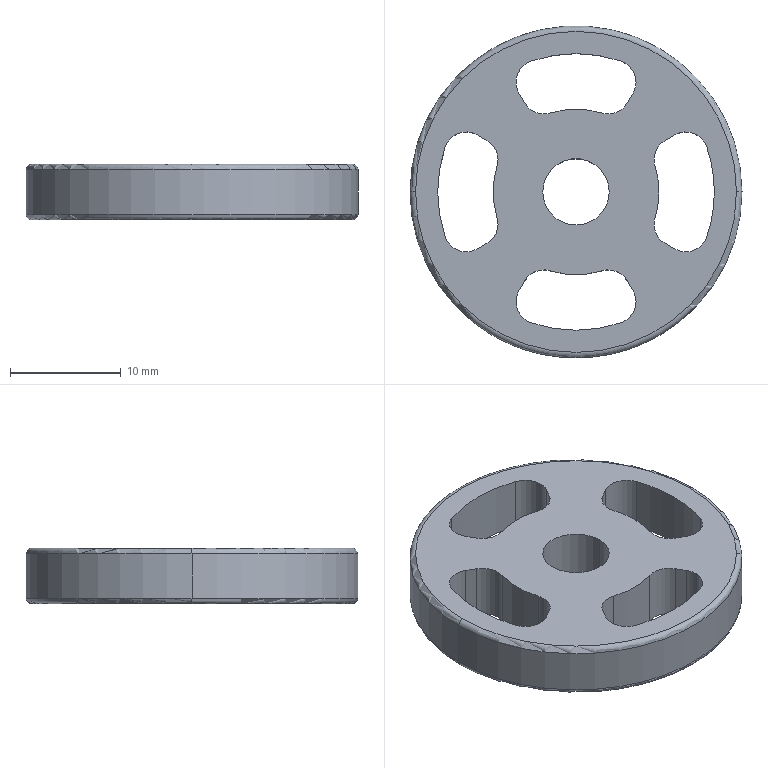Part | SolidWorks | features Extrusion 1, Fillet 1, ICE 1 | 1 solid | 48 faces | box 30 x 30 x 5 mm | volume 2405 mm3 | cylinder 34 | plane 10 | torus 4 | commonest cylinder face diameters 4 x20 15 x5 25 x5 6 x2 30 x2
STEP:
#1=CARTESIAN_POINT('',(-15.,0.,4.5));
#2=VERTEX_POINT('',#1);
#3=CARTESIAN_POINT('',(15.,0.,4.5));
#4=VERTEX_POINT('',#3);
#5=CARTESIAN_POINT('',(0.,0.,4.5));
#6=DIRECTION('',(0.,0.,-1.));
#7=DIRECTION('',(1.,0.,0.));
#8=AXIS2_PLACEMENT_3D('',#5,#6,#7);
#9=CIRCLE('',#8,15.);
#10=EDGE_CURVE('',#2,#4,#9,.T.);
#11=ORIENTED_EDGE('',*,*,#10,.F.);
#12=CARTESIAN_POINT('',(-14.5,0.,5.));
#13=VERTEX_POINT('',#12);
#14=CARTESIAN_POINT('',(-14.5,0.,4.5));
#15=DIRECTION('',(0.,1.,0.));
#16=DIRECTION('',(-1.,0.,0.));
#17=AXIS2_PLACEMENT_3D('',#14,#15,#16);
#18=CIRCLE('',#17,0.5);
#19=EDGE_CURVE('',#2,#13,#18,.T.);
#20=ORIENTED_EDGE('',*,*,#19,.T.);
#21=CARTESIAN_POINT('',(14.5,0.,5.));
#22=VERTEX_POINT('',#21);
#23=CARTESIAN_POINT('',(0.,0.,5.));
#24=DIRECTION('',(0.,0.,1.));
#25=DIRECTION('',(1.,0.,0.));
#26=AXIS2_PLACEMENT_3D('',#23,#24,#25);
#27=CIRCLE('',#26,14.5);
#28=EDGE_CURVE('',#22,#13,#27,.T.);
#29=ORIENTED_EDGE('',*,*,#28,.F.);
#30=CARTESIAN_POINT('',(14.5,0.,4.5));
#31=DIRECTION('',(0.,-1.,0.));
#32=DIRECTION('',(0.,0.,-1.));
#33=AXIS2_PLACEMENT_3D('',#30,#31,#32);
#34=CIRCLE('',#33,0.5);
#35=EDGE_CURVE('',#4,#22,#34,.T.);
#36=ORIENTED_EDGE('',*,*,#35,.F.);
#37=EDGE_LOOP('',(#11,#20,#29,#36));
#38=FACE_OUTER_BOUND('',#37,.T.);
#39=CARTESIAN_POINT('',(0.,0.,4.5));
#40=DIRECTION('',(0.,0.,1.));
#41=DIRECTION('',(1.,0.,0.));
#42=AXIS2_PLACEMENT_3D('',#39,#40,#41);
#43=TOROIDAL_SURFACE('',#42,14.5,0.5);
#44=ADVANCED_FACE('',(#38),#43,.T.);
#45=CARTESIAN_POINT('',(-14.5,0.,0.));
#46=VERTEX_POINT('',#45);
#47=CARTESIAN_POINT('',(14.5,0.,0.));
#48=VERTEX_POINT('',#47);
#49=CARTESIAN_POINT('',(0.,0.,0.));
#50=DIRECTION('',(0.,0.,-1.));
#51=DIRECTION('',(1.,0.,0.));
#52=AXIS2_PLACEMENT_3D('',#49,#50,#51);
#53=CIRCLE('',#52,14.5);
#54=EDGE_CURVE('',#46,#48,#53,.T.);
#55=ORIENTED_EDGE('',*,*,#54,.F.);
#56=CARTESIAN_POINT('',(-15.,0.,0.5));
#57=VERTEX_POINT('',#56);
#58=CARTESIAN_POINT('',(-14.5,0.,0.5));
#59=DIRECTION('',(0.,1.,0.));
#60=DIRECTION('',(-1.,0.,0.));
#61=AXIS2_PLACEMENT_3D('',#58,#59,#60);
#62=CIRCLE('',#61,0.5);
#63=EDGE_CURVE('',#46,#57,#62,.T.);
#64=ORIENTED_EDGE('',*,*,#63,.T.);
#65=CARTESIAN_POINT('',(15.,0.,0.5));
#66=VERTEX_POINT('',#65);
#67=CARTESIAN_POINT('',(0.,0.,0.5));
#68=DIRECTION('',(0.,0.,1.));
#69=DIRECTION('',(1.,0.,0.));
#70=AXIS2_PLACEMENT_3D('',#67,#68,#69);
#71=CIRCLE('',#70,15.);
#72=EDGE_CURVE('',#66,#57,#71,.T.);
#73=ORIENTED_EDGE('',*,*,#72,.F.);
#74=CARTESIAN_POINT('',(14.5,0.,0.5));
#75=DIRECTION('',(0.,-1.,0.));
#76=DIRECTION('',(0.,0.,-1.));
#77=AXIS2_PLACEMENT_3D('',#74,#75,#76);
#78=CIRCLE('',#77,0.5);
#79=EDGE_CURVE('',#48,#66,#78,.T.);
#80=ORIENTED_EDGE('',*,*,#79,.F.);
#81=EDGE_LOOP('',(#55,#64,#73,#80));
#82=FACE_OUTER_BOUND('',#81,.T.);
#83=CARTESIAN_POINT('',(0.,0.,0.5));
#84=DIRECTION('',(0.,0.,1.));
#85=DIRECTION('',(1.,0.,0.));
#86=AXIS2_PLACEMENT_3D('',#83,#84,#85);
#87=TOROIDAL_SURFACE('',#86,14.5,0.5);
#88=ADVANCED_FACE('',(#82),#87,.T.);
#89=CARTESIAN_POINT('',(5.422,9.927,0.));
#90=VERTEX_POINT('',#89);
#91=CARTESIAN_POINT('',(4.074,11.818,0.));
#92=VERTEX_POINT('',#91);
#93=CARTESIAN_POINT('',(3.422,9.927,0.));
#94=DIRECTION('',(0.,0.,1.));
#95=DIRECTION('',(1.,0.,0.));
#96=AXIS2_PLACEMENT_3D('',#93,#94,#95);
#97=CIRCLE('',#96,2.);
#98=EDGE_CURVE('',#90,#92,#97,.T.);
#99=ORIENTED_EDGE('',*,*,#98,.F.);
#100=CARTESIAN_POINT('',(5.422,9.927,5.));
#101=VERTEX_POINT('',#100);
#102=CARTESIAN_POINT('',(5.422,9.927,0.));
#103=DIRECTION('',(0.,0.,1.));
#104=VECTOR('',#103,1000.);
#105=LINE('',#102,#104);
#106=EDGE_CURVE('',#90,#101,#105,.T.);
#107=ORIENTED_EDGE('',*,*,#106,.T.);
#108=CARTESIAN_POINT('',(4.074,11.818,5.));
#109=VERTEX_POINT('',#108);
#110=CARTESIAN_POINT('',(3.422,9.927,5.));
#111=DIRECTION('',(0.,0.,1.));
#112=DIRECTION('',(1.,0.,0.));
#113=AXIS2_PLACEMENT_3D('',#110,#111,#112);
#114=CIRCLE('',#113,2.);
#115=EDGE_CURVE('',#101,#109,#114,.T.);
#116=ORIENTED_EDGE('',*,*,#115,.T.);
#117=CARTESIAN_POINT('',(4.074,11.818,0.));
#118=DIRECTION('',(0.,0.,1.));
#119=VECTOR('',#118,1000.);
#120=LINE('',#117,#119);
#121=EDGE_CURVE('',#92,#109,#120,.T.);
#122=ORIENTED_EDGE('',*,*,#121,.F.);
#123=EDGE_LOOP('',(#99,#107,#116,#122));
#124=FACE_OUTER_BOUND('',#123,.T.);
#125=CARTESIAN_POINT('',(3.422,9.927,0.));
#126=DIRECTION('',(0.,0.,1.));
#127=DIRECTION('',(1.,0.,0.));
#128=AXIS2_PLACEMENT_3D('',#125,#126,#127);
#129=CYLINDRICAL_SURFACE('',#128,2.);
#130=ADVANCED_FACE('',(#124),#129,.F.);
#131=CARTESIAN_POINT('',(7.5,0.,0.));
#132=VERTEX_POINT('',#131);
#133=CARTESIAN_POINT('',(7.139,-2.299,0.));
#134=VERTEX_POINT('',#133);
#135=CARTESIAN_POINT('',(0.,0.,0.));
#136=DIRECTION('',(0.,0.,-1.));
#137=DIRECTION('',(1.,0.,0.));
#138=AXIS2_PLACEMENT_3D('',#135,#136,#137);
#139=CIRCLE('',#138,7.5);
#140=EDGE_CURVE('',#132,#134,#139,.T.);
#141=ORIENTED_EDGE('',*,*,#140,.F.);
#142=CARTESIAN_POINT('',(7.5,0.,5.));
#143=VERTEX_POINT('',#142);
#144=CARTESIAN_POINT('',(7.5,0.,0.));
#145=DIRECTION('',(0.,0.,1.));
#146=VECTOR('',#145,1000.);
#147=LINE('',#144,#146);
#148=EDGE_CURVE('',#132,#143,#147,.T.);
#149=ORIENTED_EDGE('',*,*,#148,.T.);
#150=CARTESIAN_POINT('',(7.139,-2.299,5.));
#151=VERTEX_POINT('',#150);
#152=CARTESIAN_POINT('',(0.,0.,5.));
#153=DIRECTION('',(0.,0.,-1.));
#154=DIRECTION('',(1.,0.,0.));
#155=AXIS2_PLACEMENT_3D('',#152,#153,#154);
#156=CIRCLE('',#155,7.5);
#157=EDGE_CURVE('',#143,#151,#156,.T.);
#158=ORIENTED_EDGE('',*,*,#157,.T.);
#159=CARTESIAN_POINT('',(7.139,-2.299,0.));
#160=DIRECTION('',(0.,0.,1.));
#161=VECTOR('',#160,1000.);
#162=LINE('',#159,#161);
#163=EDGE_CURVE('',#134,#151,#162,.T.);
#164=ORIENTED_EDGE('',*,*,#163,.F.);
#165=EDGE_LOOP('',(#141,#149,#158,#164));
#166=FACE_OUTER_BOUND('',#165,.T.);
#167=CARTESIAN_POINT('',(0.,0.,0.));
#168=DIRECTION('',(0.,0.,1.));
#169=DIRECTION('',(1.,0.,0.));
#170=AXIS2_PLACEMENT_3D('',#167,#168,#169);
#171=CYLINDRICAL_SURFACE('',#170,7.5);
#172=ADVANCED_FACE('',(#166),#171,.T.);
#173=CARTESIAN_POINT('',(12.5,0.,0.));
#174=VERTEX_POINT('',#173);
#175=CARTESIAN_POINT('',(11.818,4.074,0.));
#176=VERTEX_POINT('',#175);
#177=CARTESIAN_POINT('',(0.,0.,0.));
#178=DIRECTION('',(0.,0.,1.));
#179=DIRECTION('',(1.,0.,0.));
#180=AXIS2_PLACEMENT_3D('',#177,#178,#179);
#181=CIRCLE('',#180,12.5);
#182=EDGE_CURVE('',#174,#176,#181,.T.);
#183=ORIENTED_EDGE('',*,*,#182,.F.);
#184=CARTESIAN_POINT('',(12.5,0.,5.));
#185=VERTEX_POINT('',#184);
#186=CARTESIAN_POINT('',(12.5,0.,0.));
#187=DIRECTION('',(0.,0.,1.));
#188=VECTOR('',#187,1000.);
#189=LINE('',#186,#188);
#190=EDGE_CURVE('',#174,#185,#189,.T.);
#191=ORIENTED_EDGE('',*,*,#190,.T.);
#192=CARTESIAN_POINT('',(11.818,4.074,5.));
#193=VERTEX_POINT('',#192);
#194=CARTESIAN_POINT('',(0.,0.,5.));
#195=DIRECTION('',(0.,0.,1.));
#196=DIRECTION('',(1.,0.,0.));
#197=AXIS2_PLACEMENT_3D('',#194,#195,#196);
#198=CIRCLE('',#197,12.5);
#199=EDGE_CURVE('',#185,#193,#198,.T.);
#200=ORIENTED_EDGE('',*,*,#199,.T.);
#201=CARTESIAN_POINT('',(11.818,4.074,0.));
#202=DIRECTION('',(0.,0.,1.));
#203=VECTOR('',#202,1000.);
#204=LINE('',#201,#203);
#205=EDGE_CURVE('',#176,#193,#204,.T.);
#206=ORIENTED_EDGE('',*,*,#205,.F.);
#207=EDGE_LOOP('',(#183,#191,#200,#206));
#208=FACE_OUTER_BOUND('',#207,.T.);
#209=CARTESIAN_POINT('',(0.,0.,0.));
#210=DIRECTION('',(0.,0.,1.));
#211=DIRECTION('',(1.,0.,0.));
#212=AXIS2_PLACEMENT_3D('',#209,#210,#211);
#213=CYLINDRICAL_SURFACE('',#212,12.5);
#214=ADVANCED_FACE('',(#208),#213,.F.);
#215=CARTESIAN_POINT('',(5.422,-9.927,0.));
#216=VERTEX_POINT('',#215);
#217=CARTESIAN_POINT('',(5.154,-8.927,0.));
#218=VERTEX_POINT('',#217);
#219=CARTESIAN_POINT('',(3.422,-9.927,0.));
#220=DIRECTION('',(0.,0.,1.));
#221=DIRECTION('',(-1.,0.,0.));
#222=AXIS2_PLACEMENT_3D('',#219,#220,#221);
#223=CIRCLE('',#222,2.);
#224=EDGE_CURVE('',#216,#218,#223,.T.);
#225=ORIENTED_EDGE('',*,*,#224,.F.);
#226=CARTESIAN_POINT('',(5.422,-9.927,5.));
#227=VERTEX_POINT('',#226);
#228=CARTESIAN_POINT('',(5.422,-9.927,0.));
#229=DIRECTION('',(0.,0.,1.));
#230=VECTOR('',#229,1000.);
#231=LINE('',#228,#230);
#232=EDGE_CURVE('',#216,#227,#231,.T.);
#233=ORIENTED_EDGE('',*,*,#232,.T.);
#234=CARTESIAN_POINT('',(5.154,-8.927,5.));
#235=VERTEX_POINT('',#234);
#236=CARTESIAN_POINT('',(3.422,-9.927,5.));
#237=DIRECTION('',(0.,0.,1.));
#238=DIRECTION('',(-1.,0.,0.));
#239=AXIS2_PLACEMENT_3D('',#236,#237,#238);
#240=CIRCLE('',#239,2.);
#241=EDGE_CURVE('',#227,#235,#240,.T.);
#242=ORIENTED_EDGE('',*,*,#241,.T.);
#243=CARTESIAN_POINT('',(5.154,-8.927,0.));
#244=DIRECTION('',(0.,0.,1.));
#245=VECTOR('',#244,1000.);
#246=LINE('',#243,#245);
#247=EDGE_CURVE('',#218,#235,#246,.T.);
#248=ORIENTED_EDGE('',*,*,#247,.F.);
#249=EDGE_LOOP('',(#225,#233,#242,#248));
#250=FACE_OUTER_BOUND('',#249,.T.);
#251=CARTESIAN_POINT('',(3.422,-9.927,0.));
#252=DIRECTION('',(0.,0.,1.));
#253=DIRECTION('',(1.,0.,0.));
#254=AXIS2_PLACEMENT_3D('',#251,#252,#253);
#255=CYLINDRICAL_SURFACE('',#254,2.);
#256=ADVANCED_FACE('',(#250),#255,.F.);
#257=CARTESIAN_POINT('',(-7.043,2.911,0.));
#258=VERTEX_POINT('',#257);
#259=CARTESIAN_POINT('',(-8.043,4.644,0.));
#260=VERTEX_POINT('',#259);
#261=CARTESIAN_POINT('',(-9.043,2.911,0.));
#262=DIRECTION('',(0.,0.,1.));
#263=DIRECTION('',(-1.,0.,0.));
#264=AXIS2_PLACEMENT_3D('',#261,#262,#263);
#265=CIRCLE('',#264,2.);
#266=EDGE_CURVE('',#258,#260,#265,.T.);
#267=ORIENTED_EDGE('',*,*,#266,.F.);
#268=CARTESIAN_POINT('',(-7.043,2.911,5.));
#269=VERTEX_POINT('',#268);
#270=CARTESIAN_POINT('',(-7.043,2.911,0.));
#271=DIRECTION('',(0.,0.,1.));
#272=VECTOR('',#271,1000.);
#273=LINE('',#270,#272);
#274=EDGE_CURVE('',#258,#269,#273,.T.);
#275=ORIENTED_EDGE('',*,*,#274,.T.);
#276=CARTESIAN_POINT('',(-8.043,4.644,5.));
#277=VERTEX_POINT('',#276);
#278=CARTESIAN_POINT('',(-9.043,2.911,5.));
#279=DIRECTION('',(0.,0.,1.));
#280=DIRECTION('',(-1.,0.,0.));
#281=AXIS2_PLACEMENT_3D('',#278,#279,#280);
#282=CIRCLE('',#281,2.);
#283=EDGE_CURVE('',#269,#277,#282,.T.);
#284=ORIENTED_EDGE('',*,*,#283,.T.);
#285=CARTESIAN_POINT('',(-8.043,4.644,0.));
#286=DIRECTION('',(0.,0.,1.));
#287=VECTOR('',#286,1000.);
#288=LINE('',#285,#287);
#289=EDGE_CURVE('',#260,#277,#288,.T.);
#290=ORIENTED_EDGE('',*,*,#289,.F.);
#291=EDGE_LOOP('',(#267,#275,#284,#290));
#292=FACE_OUTER_BOUND('',#291,.T.);
#293=CARTESIAN_POINT('',(-9.043,2.911,0.));
#294=DIRECTION('',(0.,0.,1.));
#295=DIRECTION('',(1.,0.,0.));
#296=AXIS2_PLACEMENT_3D('',#293,#294,#295);
#297=CYLINDRICAL_SURFACE('',#296,2.);
#298=ADVANCED_FACE('',(#292),#297,.F.);
#299=CARTESIAN_POINT('',(-7.043,-2.911,0.));
#300=VERTEX_POINT('',#299);
#301=CARTESIAN_POINT('',(-7.139,-2.299,0.));
#302=VERTEX_POINT('',#301);
#303=CARTESIAN_POINT('',(-9.043,-2.911,0.));
#304=DIRECTION('',(0.,0.,1.));
#305=DIRECTION('',(1.,0.,0.));
#306=AXIS2_PLACEMENT_3D('',#303,#304,#305);
#307=CIRCLE('',#306,2.);
#308=EDGE_CURVE('',#300,#302,#307,.T.);
#309=ORIENTED_EDGE('',*,*,#308,.F.);
#310=CARTESIAN_POINT('',(-7.043,-2.911,5.));
#311=VERTEX_POINT('',#310);
#312=CARTESIAN_POINT('',(-7.043,-2.911,0.));
#313=DIRECTION('',(0.,0.,1.));
#314=VECTOR('',#313,1000.);
#315=LINE('',#312,#314);
#316=EDGE_CURVE('',#300,#311,#315,.T.);
#317=ORIENTED_EDGE('',*,*,#316,.T.);
#318=CARTESIAN_POINT('',(-7.139,-2.299,5.));
#319=VERTEX_POINT('',#318);
#320=CARTESIAN_POINT('',(-9.043,-2.911,5.));
#321=DIRECTION('',(0.,0.,1.));
#322=DIRECTION('',(1.,0.,0.));
#323=AXIS2_PLACEMENT_3D('',#320,#321,#322);
#324=CIRCLE('',#323,2.);
#325=EDGE_CURVE('',#311,#319,#324,.T.);
#326=ORIENTED_EDGE('',*,*,#325,.T.);
#327=CARTESIAN_POINT('',(-7.139,-2.299,0.));
#328=DIRECTION('',(0.,0.,1.));
#329=VECTOR('',#328,1000.);
#330=LINE('',#327,#329);
#331=EDGE_CURVE('',#302,#319,#330,.T.);
#332=ORIENTED_EDGE('',*,*,#331,.F.);
#333=EDGE_LOOP('',(#309,#317,#326,#332));
#334=FACE_OUTER_BOUND('',#333,.T.);
#335=CARTESIAN_POINT('',(-9.043,-2.911,0.));
#336=DIRECTION('',(0.,0.,1.));
#337=DIRECTION('',(1.,0.,0.));
#338=AXIS2_PLACEMENT_3D('',#335,#336,#337);
#339=CYLINDRICAL_SURFACE('',#338,2.);
#340=ADVANCED_FACE('',(#334),#339,.F.);
#341=CARTESIAN_POINT('',(-3.,0.,5.));
#342=VERTEX_POINT('',#341);
#343=CARTESIAN_POINT('',(3.,0.,5.));
#344=VERTEX_POINT('',#343);
#345=CARTESIAN_POINT('',(0.,0.,5.));
#346=DIRECTION('',(0.,0.,1.));
#347=DIRECTION('',(1.,0.,0.));
#348=AXIS2_PLACEMENT_3D('',#345,#346,#347);
#349=CIRCLE('',#348,3.);
#350=EDGE_CURVE('',#342,#344,#349,.T.);
#351=ORIENTED_EDGE('',*,*,#350,.T.);
#352=CARTESIAN_POINT('',(3.,0.,0.));
#353=VERTEX_POINT('',#352);
#354=CARTESIAN_POINT('',(3.,0.,5.));
#355=DIRECTION('',(0.,0.,-1.));
#356=VECTOR('',#355,1000.);
#357=LINE('',#354,#356);
#358=EDGE_CURVE('',#344,#353,#357,.T.);
#359=ORIENTED_EDGE('',*,*,#358,.T.);
#360=CARTESIAN_POINT('',(-3.,0.,0.));
#361=VERTEX_POINT('',#360);
#362=CARTESIAN_POINT('',(0.,0.,0.));
#363=DIRECTION('',(0.,0.,1.));
#364=DIRECTION('',(1.,0.,0.));
#365=AXIS2_PLACEMENT_3D('',#362,#363,#364);
#366=CIRCLE('',#365,3.);
#367=EDGE_CURVE('',#361,#353,#366,.T.);
#368=ORIENTED_EDGE('',*,*,#367,.F.);
#369=CARTESIAN_POINT('',(-3.,0.,5.));
#370=DIRECTION('',(0.,0.,-1.));
#371=VECTOR('',#370,1000.);
#372=LINE('',#369,#371);
#373=EDGE_CURVE('',#342,#361,#372,.T.);
#374=ORIENTED_EDGE('',*,*,#373,.F.);
#375=EDGE_LOOP('',(#351,#359,#368,#374));
#376=FACE_OUTER_BOUND('',#375,.T.);
#377=CARTESIAN_POINT('',(0.,0.,5.));
#378=DIRECTION('',(0.,0.,-1.));
#379=DIRECTION('',(-1.,0.,0.));
#380=AXIS2_PLACEMENT_3D('',#377,#378,#379);
#381=CYLINDRICAL_SURFACE('',#380,3.);
#382=ADVANCED_FACE('',(#376),#381,.F.);
#383=ORIENTED_EDGE('',*,*,#10,.T.);
#384=CARTESIAN_POINT('',(15.,0.,5.));
#385=DIRECTION('',(0.,0.,-1.));
#386=VECTOR('',#385,1000.);
#387=LINE('',#384,#386);
#388=EDGE_CURVE('',#4,#66,#387,.T.);
#389=ORIENTED_EDGE('',*,*,#388,.T.);
#390=ORIENTED_EDGE('',*,*,#72,.T.);
#391=CARTESIAN_POINT('',(-15.,0.,5.));
#392=DIRECTION('',(0.,0.,-1.));
#393=VECTOR('',#392,1000.);
#394=LINE('',#391,#393);
#395=EDGE_CURVE('',#2,#57,#394,.T.);
#396=ORIENTED_EDGE('',*,*,#395,.F.);
#397=EDGE_LOOP('',(#383,#389,#390,#396));
#398=FACE_OUTER_BOUND('',#397,.T.);
#399=CARTESIAN_POINT('',(0.,0.,5.));
#400=DIRECTION('',(0.,0.,-1.));
#401=DIRECTION('',(-1.,0.,0.));
#402=AXIS2_PLACEMENT_3D('',#399,#400,#401);
#403=CYLINDRICAL_SURFACE('',#402,15.);
#404=ADVANCED_FACE('',(#398),#403,.T.);
#405=ORIENTED_EDGE('',*,*,#28,.T.);
#406=CARTESIAN_POINT('',(0.,0.,5.));
#407=DIRECTION('',(0.,0.,1.));
#408=DIRECTION('',(1.,0.,0.));
#409=AXIS2_PLACEMENT_3D('',#406,#407,#408);
#410=CIRCLE('',#409,14.5);
#411=EDGE_CURVE('',#13,#22,#410,.T.);
#412=ORIENTED_EDGE('',*,*,#411,.T.);
#413=EDGE_LOOP('',(#405,#412));
#414=FACE_OUTER_BOUND('',#413,.T.);
#415=CARTESIAN_POINT('',(8.043,4.644,5.));
#416=VERTEX_POINT('',#415);
#417=CARTESIAN_POINT('',(7.139,2.299,5.));
#418=VERTEX_POINT('',#417);
#419=CARTESIAN_POINT('',(9.043,2.911,5.));
#420=DIRECTION('',(0.,0.,1.));
#421=DIRECTION('',(1.,0.,0.));
#422=AXIS2_PLACEMENT_3D('',#419,#420,#421);
#423=CIRCLE('',#422,2.);
#424=EDGE_CURVE('',#416,#418,#423,.T.);
#425=ORIENTED_EDGE('',*,*,#424,.F.);
#426=CARTESIAN_POINT('',(8.927,5.154,5.));
#427=VERTEX_POINT('',#426);
#428=CARTESIAN_POINT('',(8.927,5.154,5.));
#429=DIRECTION('',(-0.866,-0.5,0.));
#430=VECTOR('',#429,1000.);
#431=LINE('',#428,#430);
#432=EDGE_CURVE('',#427,#416,#431,.T.);
#433=ORIENTED_EDGE('',*,*,#432,.F.);
#434=CARTESIAN_POINT('',(9.927,3.422,5.));
#435=DIRECTION('',(0.,0.,1.));
#436=DIRECTION('',(-1.,0.,0.));
#437=AXIS2_PLACEMENT_3D('',#434,#435,#436);
#438=CIRCLE('',#437,2.);
#439=EDGE_CURVE('',#193,#427,#438,.T.);
#440=ORIENTED_EDGE('',*,*,#439,.F.);
#441=ORIENTED_EDGE('',*,*,#199,.F.);
#442=CARTESIAN_POINT('',(11.818,-4.074,5.));
#443=VERTEX_POINT('',#442);
#444=CARTESIAN_POINT('',(0.,0.,5.));
#445=DIRECTION('',(0.,0.,1.));
#446=DIRECTION('',(1.,0.,0.));
#447=AXIS2_PLACEMENT_3D('',#444,#445,#446);
#448=CIRCLE('',#447,12.5);
#449=EDGE_CURVE('',#443,#185,#448,.T.);
#450=ORIENTED_EDGE('',*,*,#449,.F.);
#451=CARTESIAN_POINT('',(8.927,-5.154,5.));
#452=VERTEX_POINT('',#451);
#453=CARTESIAN_POINT('',(9.927,-3.422,5.));
#454=DIRECTION('',(0.,0.,1.));
#455=DIRECTION('',(1.,0.,0.));
#456=AXIS2_PLACEMENT_3D('',#453,#454,#455);
#457=CIRCLE('',#456,2.);
#458=EDGE_CURVE('',#452,#443,#457,.T.);
#459=ORIENTED_EDGE('',*,*,#458,.F.);
#460=CARTESIAN_POINT('',(8.043,-4.644,5.));
#461=VERTEX_POINT('',#460);
#462=CARTESIAN_POINT('',(8.927,-5.154,5.));
#463=DIRECTION('',(0.866,-0.5,0.));
#464=VECTOR('',#463,1000.);
#465=LINE('',#462,#464);
#466=EDGE_CURVE('',#461,#452,#465,.T.);
#467=ORIENTED_EDGE('',*,*,#466,.F.);
#468=CARTESIAN_POINT('',(9.043,-2.911,5.));
#469=DIRECTION('',(0.,0.,1.));
#470=DIRECTION('',(-1.,0.,0.));
#471=AXIS2_PLACEMENT_3D('',#468,#469,#470);
#472=CIRCLE('',#471,2.);
#473=EDGE_CURVE('',#151,#461,#472,.T.);
#474=ORIENTED_EDGE('',*,*,#473,.F.);
#475=ORIENTED_EDGE('',*,*,#157,.F.);
#476=CARTESIAN_POINT('',(0.,0.,5.));
#477=DIRECTION('',(0.,0.,-1.));
#478=DIRECTION('',(1.,0.,0.));
#479=AXIS2_PLACEMENT_3D('',#476,#477,#478);
#480=CIRCLE('',#479,7.5);
#481=EDGE_CURVE('',#418,#143,#480,.T.);
#482=ORIENTED_EDGE('',*,*,#481,.F.);
#483=EDGE_LOOP('',(#425,#433,#440,#441,#450,#459,#467,#474,#475,#482));
#484=FACE_BOUND('',#483,.T.);
#485=CARTESIAN_POINT('',(-8.043,-4.644,5.));
#486=VERTEX_POINT('',#485);
#487=CARTESIAN_POINT('',(-9.043,-2.911,5.));
#488=DIRECTION('',(0.,0.,1.));
#489=DIRECTION('',(1.,0.,0.));
#490=AXIS2_PLACEMENT_3D('',#487,#488,#489);
#491=CIRCLE('',#490,2.);
#492=EDGE_CURVE('',#486,#311,#491,.T.);
#493=ORIENTED_EDGE('',*,*,#492,.F.);
#494=CARTESIAN_POINT('',(-8.927,-5.154,5.));
#495=VERTEX_POINT('',#494);
#496=CARTESIAN_POINT('',(-8.927,-5.154,5.));
#497=DIRECTION('',(0.866,0.5,0.));
#498=VECTOR('',#497,1000.);
#499=LINE('',#496,#498);
#500=EDGE_CURVE('',#495,#486,#499,.T.);
#501=ORIENTED_EDGE('',*,*,#500,.F.);
#502=CARTESIAN_POINT('',(-11.818,-4.074,5.));
#503=VERTEX_POINT('',#502);
#504=CARTESIAN_POINT('',(-9.927,-3.422,5.));
#505=DIRECTION('',(0.,0.,1.));
#506=DIRECTION('',(-1.,0.,0.));
#507=AXIS2_PLACEMENT_3D('',#504,#505,#506);
#508=CIRCLE('',#507,2.);
#509=EDGE_CURVE('',#503,#495,#508,.T.);
#510=ORIENTED_EDGE('',*,*,#509,.F.);
#511=CARTESIAN_POINT('',(-11.818,4.074,5.));
#512=VERTEX_POINT('',#511);
#513=CARTESIAN_POINT('',(0.,0.,5.));
#514=DIRECTION('',(0.,0.,1.));
#515=DIRECTION('',(1.,0.,0.));
#516=AXIS2_PLACEMENT_3D('',#513,#514,#515);
#517=CIRCLE('',#516,12.5);
#518=EDGE_CURVE('',#512,#503,#517,.T.);
#519=ORIENTED_EDGE('',*,*,#518,.F.);
#520=CARTESIAN_POINT('',(-8.927,5.154,5.));
#521=VERTEX_POINT('',#520);
#522=CARTESIAN_POINT('',(-9.927,3.422,5.));
#523=DIRECTION('',(0.,0.,1.));
#524=DIRECTION('',(1.,0.,0.));
#525=AXIS2_PLACEMENT_3D('',#522,#523,#524);
#526=CIRCLE('',#525,2.);
#527=EDGE_CURVE('',#521,#512,#526,.T.);
#528=ORIENTED_EDGE('',*,*,#527,.F.);
#529=CARTESIAN_POINT('',(-8.927,5.154,5.));
#530=DIRECTION('',(-0.866,0.5,0.));
#531=VECTOR('',#530,1000.);
#532=LINE('',#529,#531);
#533=EDGE_CURVE('',#277,#521,#532,.T.);
#534=ORIENTED_EDGE('',*,*,#533,.F.);
#535=ORIENTED_EDGE('',*,*,#283,.F.);
#536=CARTESIAN_POINT('',(-7.139,2.299,5.));
#537=VERTEX_POINT('',#536);
#538=CARTESIAN_POINT('',(-9.043,2.911,5.));
#539=DIRECTION('',(0.,0.,1.));
#540=DIRECTION('',(-1.,0.,0.));
#541=AXIS2_PLACEMENT_3D('',#538,#539,#540);
#542=CIRCLE('',#541,2.);
#543=EDGE_CURVE('',#537,#269,#542,.T.);
#544=ORIENTED_EDGE('',*,*,#543,.F.);
#545=CARTESIAN_POINT('',(0.,0.,5.));
#546=DIRECTION('',(0.,0.,-1.));
#547=DIRECTION('',(1.,0.,0.));
#548=AXIS2_PLACEMENT_3D('',#545,#546,#547);
#549=CIRCLE('',#548,7.5);
#550=EDGE_CURVE('',#319,#537,#549,.T.);
#551=ORIENTED_EDGE('',*,*,#550,.F.);
#552=ORIENTED_EDGE('',*,*,#325,.F.);
#553=EDGE_LOOP('',(#493,#501,#510,#519,#528,#534,#535,#544,#551,#552));
#554=FACE_BOUND('',#553,.T.);
#555=ORIENTED_EDGE('',*,*,#350,.F.);
#556=CARTESIAN_POINT('',(0.,0.,5.));
#557=DIRECTION('',(0.,0.,1.));
#558=DIRECTION('',(1.,0.,0.));
#559=AXIS2_PLACEMENT_3D('',#556,#557,#558);
#560=CIRCLE('',#559,3.);
#561=EDGE_CURVE('',#344,#342,#560,.T.);
#562=ORIENTED_EDGE('',*,*,#561,.F.);
#563=EDGE_LOOP('',(#555,#562));
#564=FACE_BOUND('',#563,.T.);
#565=CARTESIAN_POINT('',(4.644,-8.043,5.));
#566=VERTEX_POINT('',#565);
#567=CARTESIAN_POINT('',(2.299,-7.139,5.));
#568=VERTEX_POINT('',#567);
#569=CARTESIAN_POINT('',(2.911,-9.043,5.));
#570=DIRECTION('',(0.,0.,1.));
#571=DIRECTION('',(1.,0.,0.));
#572=AXIS2_PLACEMENT_3D('',#569,#570,#571);
#573=CIRCLE('',#572,2.);
#574=EDGE_CURVE('',#566,#568,#573,.T.);
#575=ORIENTED_EDGE('',*,*,#574,.F.);
#576=CARTESIAN_POINT('',(5.154,-8.927,5.));
#577=DIRECTION('',(-0.5,0.866,0.));
#578=VECTOR('',#577,1000.);
#579=LINE('',#576,#578);
#580=EDGE_CURVE('',#235,#566,#579,.T.);
#581=ORIENTED_EDGE('',*,*,#580,.F.);
#582=ORIENTED_EDGE('',*,*,#241,.F.);
#583=CARTESIAN_POINT('',(4.074,-11.818,5.));
#584=VERTEX_POINT('',#583);
#585=CARTESIAN_POINT('',(3.422,-9.927,5.));
#586=DIRECTION('',(0.,0.,1.));
#587=DIRECTION('',(-1.,0.,0.));
#588=AXIS2_PLACEMENT_3D('',#585,#586,#587);
#589=CIRCLE('',#588,2.);
#590=EDGE_CURVE('',#584,#227,#589,.T.);
#591=ORIENTED_EDGE('',*,*,#590,.F.);
#592=CARTESIAN_POINT('',(-4.074,-11.818,5.));
#593=VERTEX_POINT('',#592);
#594=CARTESIAN_POINT('',(0.,0.,5.));
#595=DIRECTION('',(0.,0.,1.));
#596=DIRECTION('',(1.,0.,0.));
#597=AXIS2_PLACEMENT_3D('',#594,#595,#596);
#598=CIRCLE('',#597,12.5);
#599=EDGE_CURVE('',#593,#584,#598,.T.);
#600=ORIENTED_EDGE('',*,*,#599,.F.);
#601=CARTESIAN_POINT('',(-5.154,-8.927,5.));
#602=VERTEX_POINT('',#601);
#603=CARTESIAN_POINT('',(-3.422,-9.927,5.));
#604=DIRECTION('',(0.,0.,1.));
#605=DIRECTION('',(1.,0.,0.));
#606=AXIS2_PLACEMENT_3D('',#603,#604,#605);
#607=CIRCLE('',#606,2.);
#608=EDGE_CURVE('',#602,#593,#607,.T.);
#609=ORIENTED_EDGE('',*,*,#608,.F.);
#610=CARTESIAN_POINT('',(-4.644,-8.043,5.));
#611=VERTEX_POINT('',#610);
#612=CARTESIAN_POINT('',(-5.154,-8.927,5.));
#613=DIRECTION('',(-0.5,-0.866,0.));
#614=VECTOR('',#613,1000.);
#615=LINE('',#612,#614);
#616=EDGE_CURVE('',#611,#602,#615,.T.);
#617=ORIENTED_EDGE('',*,*,#616,.F.);
#618=CARTESIAN_POINT('',(-2.299,-7.139,5.));
#619=VERTEX_POINT('',#618);
#620=CARTESIAN_POINT('',(-2.911,-9.043,5.));
#621=DIRECTION('',(0.,0.,1.));
#622=DIRECTION('',(-1.,0.,0.));
#623=AXIS2_PLACEMENT_3D('',#620,#621,#622);
#624=CIRCLE('',#623,2.);
#625=EDGE_CURVE('',#619,#611,#624,.T.);
#626=ORIENTED_EDGE('',*,*,#625,.F.);
#627=CARTESIAN_POINT('',(0.,0.,5.));
#628=DIRECTION('',(0.,0.,-1.));
#629=DIRECTION('',(1.,0.,0.));
#630=AXIS2_PLACEMENT_3D('',#627,#628,#629);
#631=CIRCLE('',#630,7.5);
#632=EDGE_CURVE('',#568,#619,#631,.T.);
#633=ORIENTED_EDGE('',*,*,#632,.F.);
#634=EDGE_LOOP('',(#575,#581,#582,#591,#600,#609,#617,#626,#633));
#635=FACE_BOUND('',#634,.T.);
#636=CARTESIAN_POINT('',(-4.644,8.043,5.));
#637=VERTEX_POINT('',#636);
#638=CARTESIAN_POINT('',(-2.299,7.139,5.));
#639=VERTEX_POINT('',#638);
#640=CARTESIAN_POINT('',(-2.911,9.043,5.));
#641=DIRECTION('',(0.,0.,1.));
#642=DIRECTION('',(1.,0.,0.));
#643=AXIS2_PLACEMENT_3D('',#640,#641,#642);
#644=CIRCLE('',#643,2.);
#645=EDGE_CURVE('',#637,#639,#644,.T.);
#646=ORIENTED_EDGE('',*,*,#645,.F.);
#647=CARTESIAN_POINT('',(-5.154,8.927,5.));
#648=VERTEX_POINT('',#647);
#649=CARTESIAN_POINT('',(-5.154,8.927,5.));
#650=DIRECTION('',(0.5,-0.866,0.));
#651=VECTOR('',#650,1000.);
#652=LINE('',#649,#651);
#653=EDGE_CURVE('',#648,#637,#652,.T.);
#654=ORIENTED_EDGE('',*,*,#653,.F.);
#655=CARTESIAN_POINT('',(-4.074,11.818,5.));
#656=VERTEX_POINT('',#655);
#657=CARTESIAN_POINT('',(-3.422,9.927,5.));
#658=DIRECTION('',(0.,0.,1.));
#659=DIRECTION('',(-1.,0.,0.));
#660=AXIS2_PLACEMENT_3D('',#657,#658,#659);
#661=CIRCLE('',#660,2.);
#662=EDGE_CURVE('',#656,#648,#661,.T.);
#663=ORIENTED_EDGE('',*,*,#662,.F.);
#664=CARTESIAN_POINT('',(0.,0.,5.));
#665=DIRECTION('',(0.,0.,1.));
#666=DIRECTION('',(1.,0.,0.));
#667=AXIS2_PLACEMENT_3D('',#664,#665,#666);
#668=CIRCLE('',#667,12.5);
#669=EDGE_CURVE('',#109,#656,#668,.T.);
#670=ORIENTED_EDGE('',*,*,#669,.F.);
#671=ORIENTED_EDGE('',*,*,#115,.F.);
#672=CARTESIAN_POINT('',(5.154,8.927,5.));
#673=VERTEX_POINT('',#672);
#674=CARTESIAN_POINT('',(3.422,9.927,5.));
#675=DIRECTION('',(0.,0.,1.));
#676=DIRECTION('',(1.,0.,0.));
#677=AXIS2_PLACEMENT_3D('',#674,#675,#676);
#678=CIRCLE('',#677,2.);
#679=EDGE_CURVE('',#673,#101,#678,.T.);
#680=ORIENTED_EDGE('',*,*,#679,.F.);
#681=CARTESIAN_POINT('',(4.644,8.043,5.));
#682=VERTEX_POINT('',#681);
#683=CARTESIAN_POINT('',(5.154,8.927,5.));
#684=DIRECTION('',(0.5,0.866,0.));
#685=VECTOR('',#684,1000.);
#686=LINE('',#683,#685);
#687=EDGE_CURVE('',#682,#673,#686,.T.);
#688=ORIENTED_EDGE('',*,*,#687,.F.);
#689=CARTESIAN_POINT('',(2.299,7.139,5.));
#690=VERTEX_POINT('',#689);
#691=CARTESIAN_POINT('',(2.911,9.043,5.));
#692=DIRECTION('',(0.,0.,1.));
#693=DIRECTION('',(-1.,0.,0.));
#694=AXIS2_PLACEMENT_3D('',#691,#692,#693);
#695=CIRCLE('',#694,2.);
#696=EDGE_CURVE('',#690,#682,#695,.T.);
#697=ORIENTED_EDGE('',*,*,#696,.F.);
#698=CARTESIAN_POINT('',(0.,0.,5.));
#699=DIRECTION('',(0.,0.,-1.));
#700=DIRECTION('',(1.,0.,0.));
#701=AXIS2_PLACEMENT_3D('',#698,#699,#700);
#702=CIRCLE('',#701,7.5);
#703=EDGE_CURVE('',#639,#690,#702,.T.);
#704=ORIENTED_EDGE('',*,*,#703,.F.);
#705=EDGE_LOOP('',(#646,#654,#663,#670,#671,#680,#688,#697,#704));
#706=FACE_BOUND('',#705,.T.);
#707=CARTESIAN_POINT('',(0.,0.,5.));
#708=DIRECTION('',(0.,0.,1.));
#709=DIRECTION('',(1.,0.,0.));
#710=AXIS2_PLACEMENT_3D('',#707,#708,#709);
#711=PLANE('',#710);
#712=ADVANCED_FACE('',(#414,#484,#554,#564,#635,#706),#711,.T.);
#713=CARTESIAN_POINT('',(0.,0.,0.));
#714=DIRECTION('',(0.,0.,-1.));
#715=DIRECTION('',(1.,0.,0.));
#716=AXIS2_PLACEMENT_3D('',#713,#714,#715);
#717=CIRCLE('',#716,14.5);
#718=EDGE_CURVE('',#48,#46,#717,.T.);
#719=ORIENTED_EDGE('',*,*,#718,.T.);
#720=ORIENTED_EDGE('',*,*,#54,.T.);
#721=EDGE_LOOP('',(#719,#720));
#722=FACE_OUTER_BOUND('',#721,.T.);
#723=ORIENTED_EDGE('',*,*,#367,.T.);
#724=CARTESIAN_POINT('',(0.,0.,0.));
#725=DIRECTION('',(0.,0.,1.));
#726=DIRECTION('',(1.,0.,0.));
#727=AXIS2_PLACEMENT_3D('',#724,#725,#726);
#728=CIRCLE('',#727,3.);
#729=EDGE_CURVE('',#353,#361,#728,.T.);
#730=ORIENTED_EDGE('',*,*,#729,.T.);
#731=EDGE_LOOP('',(#723,#730));
#732=FACE_BOUND('',#731,.T.);
#733=CARTESIAN_POINT('',(-8.927,-5.154,0.));
#734=VERTEX_POINT('',#733);
#735=CARTESIAN_POINT('',(-8.043,-4.644,0.));
#736=VERTEX_POINT('',#735);
#737=CARTESIAN_POINT('',(-8.927,-5.154,0.));
#738=DIRECTION('',(0.866,0.5,0.));
#739=VECTOR('',#738,1000.);
#740=LINE('',#737,#739);
#741=EDGE_CURVE('',#734,#736,#740,.T.);
#742=ORIENTED_EDGE('',*,*,#741,.T.);
#743=CARTESIAN_POINT('',(-9.043,-2.911,0.));
#744=DIRECTION('',(0.,0.,1.));
#745=DIRECTION('',(1.,0.,0.));
#746=AXIS2_PLACEMENT_3D('',#743,#744,#745);
#747=CIRCLE('',#746,2.);
#748=EDGE_CURVE('',#736,#300,#747,.T.);
#749=ORIENTED_EDGE('',*,*,#748,.T.);
#750=ORIENTED_EDGE('',*,*,#308,.T.);
#751=CARTESIAN_POINT('',(-7.139,2.299,0.));
#752=VERTEX_POINT('',#751);
#753=CARTESIAN_POINT('',(0.,0.,0.));
#754=DIRECTION('',(0.,0.,-1.));
#755=DIRECTION('',(1.,0.,0.));
#756=AXIS2_PLACEMENT_3D('',#753,#754,#755);
#757=CIRCLE('',#756,7.5);
#758=EDGE_CURVE('',#302,#752,#757,.T.);
#759=ORIENTED_EDGE('',*,*,#758,.T.);
#760=CARTESIAN_POINT('',(-9.043,2.911,0.));
#761=DIRECTION('',(0.,0.,1.));
#762=DIRECTION('',(-1.,0.,0.));
#763=AXIS2_PLACEMENT_3D('',#760,#761,#762);
#764=CIRCLE('',#763,2.);
#765=EDGE_CURVE('',#752,#258,#764,.T.);
#766=ORIENTED_EDGE('',*,*,#765,.T.);
#767=ORIENTED_EDGE('',*,*,#266,.T.);
#768=CARTESIAN_POINT('',(-8.927,5.154,0.));
#769=VERTEX_POINT('',#768);
#770=CARTESIAN_POINT('',(-8.927,5.154,0.));
#771=DIRECTION('',(-0.866,0.5,0.));
#772=VECTOR('',#771,1000.);
#773=LINE('',#770,#772);
#774=EDGE_CURVE('',#260,#769,#773,.T.);
#775=ORIENTED_EDGE('',*,*,#774,.T.);
#776=CARTESIAN_POINT('',(-11.818,4.074,0.));
#777=VERTEX_POINT('',#776);
#778=CARTESIAN_POINT('',(-9.927,3.422,0.));
#779=DIRECTION('',(0.,0.,1.));
#780=DIRECTION('',(1.,0.,0.));
#781=AXIS2_PLACEMENT_3D('',#778,#779,#780);
#782=CIRCLE('',#781,2.);
#783=EDGE_CURVE('',#769,#777,#782,.T.);
#784=ORIENTED_EDGE('',*,*,#783,.T.);
#785=CARTESIAN_POINT('',(-11.818,-4.074,0.));
#786=VERTEX_POINT('',#785);
#787=CARTESIAN_POINT('',(0.,0.,0.));
#788=DIRECTION('',(0.,0.,1.));
#789=DIRECTION('',(1.,0.,0.));
#790=AXIS2_PLACEMENT_3D('',#787,#788,#789);
#791=CIRCLE('',#790,12.5);
#792=EDGE_CURVE('',#777,#786,#791,.T.);
#793=ORIENTED_EDGE('',*,*,#792,.T.);
#794=CARTESIAN_POINT('',(-9.927,-3.422,0.));
#795=DIRECTION('',(0.,0.,1.));
#796=DIRECTION('',(-1.,0.,0.));
#797=AXIS2_PLACEMENT_3D('',#794,#795,#796);
#798=CIRCLE('',#797,2.);
#799=EDGE_CURVE('',#786,#734,#798,.T.);
#800=ORIENTED_EDGE('',*,*,#799,.T.);
#801=EDGE_LOOP('',(#742,#749,#750,#759,#766,#767,#775,#784,#793,#800));
#802=FACE_BOUND('',#801,.T.);
#803=CARTESIAN_POINT('',(4.644,-8.043,0.));
#804=VERTEX_POINT('',#803);
#805=CARTESIAN_POINT('',(5.154,-8.927,0.));
#806=DIRECTION('',(-0.5,0.866,0.));
#807=VECTOR('',#806,1000.);
#808=LINE('',#805,#807);
#809=EDGE_CURVE('',#218,#804,#808,.T.);
#810=ORIENTED_EDGE('',*,*,#809,.T.);
#811=CARTESIAN_POINT('',(2.299,-7.139,0.));
#812=VERTEX_POINT('',#811);
#813=CARTESIAN_POINT('',(2.911,-9.043,0.));
#814=DIRECTION('',(0.,0.,1.));
#815=DIRECTION('',(1.,0.,0.));
#816=AXIS2_PLACEMENT_3D('',#813,#814,#815);
#817=CIRCLE('',#816,2.);
#818=EDGE_CURVE('',#804,#812,#817,.T.);
#819=ORIENTED_EDGE('',*,*,#818,.T.);
#820=CARTESIAN_POINT('',(-2.299,-7.139,0.));
#821=VERTEX_POINT('',#820);
#822=CARTESIAN_POINT('',(0.,0.,0.));
#823=DIRECTION('',(0.,0.,-1.));
#824=DIRECTION('',(1.,0.,0.));
#825=AXIS2_PLACEMENT_3D('',#822,#823,#824);
#826=CIRCLE('',#825,7.5);
#827=EDGE_CURVE('',#812,#821,#826,.T.);
#828=ORIENTED_EDGE('',*,*,#827,.T.);
#829=CARTESIAN_POINT('',(-4.644,-8.043,0.));
#830=VERTEX_POINT('',#829);
#831=CARTESIAN_POINT('',(-2.911,-9.043,0.));
#832=DIRECTION('',(0.,0.,1.));
#833=DIRECTION('',(-1.,0.,0.));
#834=AXIS2_PLACEMENT_3D('',#831,#832,#833);
#835=CIRCLE('',#834,2.);
#836=EDGE_CURVE('',#821,#830,#835,.T.);
#837=ORIENTED_EDGE('',*,*,#836,.T.);
#838=CARTESIAN_POINT('',(-5.154,-8.927,0.));
#839=VERTEX_POINT('',#838);
#840=CARTESIAN_POINT('',(-5.154,-8.927,0.));
#841=DIRECTION('',(-0.5,-0.866,0.));
#842=VECTOR('',#841,1000.);
#843=LINE('',#840,#842);
#844=EDGE_CURVE('',#830,#839,#843,.T.);
#845=ORIENTED_EDGE('',*,*,#844,.T.);
#846=CARTESIAN_POINT('',(-4.074,-11.818,0.));
#847=VERTEX_POINT('',#846);
#848=CARTESIAN_POINT('',(-3.422,-9.927,0.));
#849=DIRECTION('',(0.,0.,1.));
#850=DIRECTION('',(1.,0.,0.));
#851=AXIS2_PLACEMENT_3D('',#848,#849,#850);
#852=CIRCLE('',#851,2.);
#853=EDGE_CURVE('',#839,#847,#852,.T.);
#854=ORIENTED_EDGE('',*,*,#853,.T.);
#855=CARTESIAN_POINT('',(4.074,-11.818,0.));
#856=VERTEX_POINT('',#855);
#857=CARTESIAN_POINT('',(0.,0.,0.));
#858=DIRECTION('',(0.,0.,1.));
#859=DIRECTION('',(1.,0.,0.));
#860=AXIS2_PLACEMENT_3D('',#857,#858,#859);
#861=CIRCLE('',#860,12.5);
#862=EDGE_CURVE('',#847,#856,#861,.T.);
#863=ORIENTED_EDGE('',*,*,#862,.T.);
#864=CARTESIAN_POINT('',(3.422,-9.927,0.));
#865=DIRECTION('',(0.,0.,1.));
#866=DIRECTION('',(-1.,0.,0.));
#867=AXIS2_PLACEMENT_3D('',#864,#865,#866);
#868=CIRCLE('',#867,2.);
#869=EDGE_CURVE('',#856,#216,#868,.T.);
#870=ORIENTED_EDGE('',*,*,#869,.T.);
#871=ORIENTED_EDGE('',*,*,#224,.T.);
#872=EDGE_LOOP('',(#810,#819,#828,#837,#845,#854,#863,#870,#871));
#873=FACE_BOUND('',#872,.T.);
#874=CARTESIAN_POINT('',(8.927,5.154,0.));
#875=VERTEX_POINT('',#874);
#876=CARTESIAN_POINT('',(8.043,4.644,0.));
#877=VERTEX_POINT('',#876);
#878=CARTESIAN_POINT('',(8.927,5.154,0.));
#879=DIRECTION('',(-0.866,-0.5,0.));
#880=VECTOR('',#879,1000.);
#881=LINE('',#878,#880);
#882=EDGE_CURVE('',#875,#877,#881,.T.);
#883=ORIENTED_EDGE('',*,*,#882,.T.);
#884=CARTESIAN_POINT('',(7.139,2.299,0.));
#885=VERTEX_POINT('',#884);
#886=CARTESIAN_POINT('',(9.043,2.911,0.));
#887=DIRECTION('',(0.,0.,1.));
#888=DIRECTION('',(1.,0.,0.));
#889=AXIS2_PLACEMENT_3D('',#886,#887,#888);
#890=CIRCLE('',#889,2.);
#891=EDGE_CURVE('',#877,#885,#890,.T.);
#892=ORIENTED_EDGE('',*,*,#891,.T.);
#893=CARTESIAN_POINT('',(0.,0.,0.));
#894=DIRECTION('',(0.,0.,-1.));
#895=DIRECTION('',(1.,0.,0.));
#896=AXIS2_PLACEMENT_3D('',#893,#894,#895);
#897=CIRCLE('',#896,7.5);
#898=EDGE_CURVE('',#885,#132,#897,.T.);
#899=ORIENTED_EDGE('',*,*,#898,.T.);
#900=ORIENTED_EDGE('',*,*,#140,.T.);
#901=CARTESIAN_POINT('',(8.043,-4.644,0.));
#902=VERTEX_POINT('',#901);
#903=CARTESIAN_POINT('',(9.043,-2.911,0.));
#904=DIRECTION('',(0.,0.,1.));
#905=DIRECTION('',(-1.,0.,0.));
#906=AXIS2_PLACEMENT_3D('',#903,#904,#905);
#907=CIRCLE('',#906,2.);
#908=EDGE_CURVE('',#134,#902,#907,.T.);
#909=ORIENTED_EDGE('',*,*,#908,.T.);
#910=CARTESIAN_POINT('',(8.927,-5.154,0.));
#911=VERTEX_POINT('',#910);
#912=CARTESIAN_POINT('',(8.927,-5.154,0.));
#913=DIRECTION('',(0.866,-0.5,0.));
#914=VECTOR('',#913,1000.);
#915=LINE('',#912,#914);
#916=EDGE_CURVE('',#902,#911,#915,.T.);
#917=ORIENTED_EDGE('',*,*,#916,.T.);
#918=CARTESIAN_POINT('',(11.818,-4.074,0.));
#919=VERTEX_POINT('',#918);
#920=CARTESIAN_POINT('',(9.927,-3.422,0.));
#921=DIRECTION('',(0.,0.,1.));
#922=DIRECTION('',(1.,0.,0.));
#923=AXIS2_PLACEMENT_3D('',#920,#921,#922);
#924=CIRCLE('',#923,2.);
#925=EDGE_CURVE('',#911,#919,#924,.T.);
#926=ORIENTED_EDGE('',*,*,#925,.T.);
#927=CARTESIAN_POINT('',(0.,0.,0.));
#928=DIRECTION('',(0.,0.,1.));
#929=DIRECTION('',(1.,0.,0.));
#930=AXIS2_PLACEMENT_3D('',#927,#928,#929);
#931=CIRCLE('',#930,12.5);
#932=EDGE_CURVE('',#919,#174,#931,.T.);
#933=ORIENTED_EDGE('',*,*,#932,.T.);
#934=ORIENTED_EDGE('',*,*,#182,.T.);
#935=CARTESIAN_POINT('',(9.927,3.422,0.));
#936=DIRECTION('',(0.,0.,1.));
#937=DIRECTION('',(-1.,0.,0.));
#938=AXIS2_PLACEMENT_3D('',#935,#936,#937);
#939=CIRCLE('',#938,2.);
#940=EDGE_CURVE('',#176,#875,#939,.T.);
#941=ORIENTED_EDGE('',*,*,#940,.T.);
#942=EDGE_LOOP('',(#883,#892,#899,#900,#909,#917,#926,#933,#934,#941));
#943=FACE_BOUND('',#942,.T.);
#944=CARTESIAN_POINT('',(-5.154,8.927,0.));
#945=VERTEX_POINT('',#944);
#946=CARTESIAN_POINT('',(-4.644,8.043,0.));
#947=VERTEX_POINT('',#946);
#948=CARTESIAN_POINT('',(-5.154,8.927,0.));
#949=DIRECTION('',(0.5,-0.866,0.));
#950=VECTOR('',#949,1000.);
#951=LINE('',#948,#950);
#952=EDGE_CURVE('',#945,#947,#951,.T.);
#953=ORIENTED_EDGE('',*,*,#952,.T.);
#954=CARTESIAN_POINT('',(-2.299,7.139,0.));
#955=VERTEX_POINT('',#954);
#956=CARTESIAN_POINT('',(-2.911,9.043,0.));
#957=DIRECTION('',(0.,0.,1.));
#958=DIRECTION('',(1.,0.,0.));
#959=AXIS2_PLACEMENT_3D('',#956,#957,#958);
#960=CIRCLE('',#959,2.);
#961=EDGE_CURVE('',#947,#955,#960,.T.);
#962=ORIENTED_EDGE('',*,*,#961,.T.);
#963=CARTESIAN_POINT('',(2.299,7.139,0.));
#964=VERTEX_POINT('',#963);
#965=CARTESIAN_POINT('',(0.,0.,0.));
#966=DIRECTION('',(0.,0.,-1.));
#967=DIRECTION('',(1.,0.,0.));
#968=AXIS2_PLACEMENT_3D('',#965,#966,#967);
#969=CIRCLE('',#968,7.5);
#970=EDGE_CURVE('',#955,#964,#969,.T.);
#971=ORIENTED_EDGE('',*,*,#970,.T.);
#972=CARTESIAN_POINT('',(4.644,8.043,0.));
#973=VERTEX_POINT('',#972);
#974=CARTESIAN_POINT('',(2.911,9.043,0.));
#975=DIRECTION('',(0.,0.,1.));
#976=DIRECTION('',(-1.,0.,0.));
#977=AXIS2_PLACEMENT_3D('',#974,#975,#976);
#978=CIRCLE('',#977,2.);
#979=EDGE_CURVE('',#964,#973,#978,.T.);
#980=ORIENTED_EDGE('',*,*,#979,.T.);
#981=CARTESIAN_POINT('',(5.154,8.927,0.));
#982=VERTEX_POINT('',#981);
#983=CARTESIAN_POINT('',(5.154,8.927,0.));
#984=DIRECTION('',(0.5,0.866,0.));
#985=VECTOR('',#984,1000.);
#986=LINE('',#983,#985);
#987=EDGE_CURVE('',#973,#982,#986,.T.);
#988=ORIENTED_EDGE('',*,*,#987,.T.);
#989=CARTESIAN_POINT('',(3.422,9.927,0.));
#990=DIRECTION('',(0.,0.,1.));
#991=DIRECTION('',(1.,0.,0.));
#992=AXIS2_PLACEMENT_3D('',#989,#990,#991);
#993=CIRCLE('',#992,2.);
#994=EDGE_CURVE('',#982,#90,#993,.T.);
#995=ORIENTED_EDGE('',*,*,#994,.T.);
#996=ORIENTED_EDGE('',*,*,#98,.T.);
#997=CARTESIAN_POINT('',(-4.074,11.818,0.));
#998=VERTEX_POINT('',#997);
#999=CARTESIAN_POINT('',(0.,0.,0.));
#1000=DIRECTION('',(0.,0.,1.));
#1001=DIRECTION('',(1.,0.,0.));
#1002=AXIS2_PLACEMENT_3D('',#999,#1000,#1001);
#1003=CIRCLE('',#1002,12.5);
#1004=EDGE_CURVE('',#92,#998,#1003,.T.);
#1005=ORIENTED_EDGE('',*,*,#1004,.T.);
#1006=CARTESIAN_POINT('',(-3.422,9.927,0.));
#1007=DIRECTION('',(0.,0.,1.));
#1008=DIRECTION('',(-1.,0.,0.));
#1009=AXIS2_PLACEMENT_3D('',#1006,#1007,#1008);
#1010=CIRCLE('',#1009,2.);
#1011=EDGE_CURVE('',#998,#945,#1010,.T.);
#1012=ORIENTED_EDGE('',*,*,#1011,.T.);
#1013=EDGE_LOOP('',(#953,#962,#971,#980,#988,#995,#996,#1005,#1012));
#1014=FACE_BOUND('',#1013,.T.);
#1015=CARTESIAN_POINT('',(0.,0.,0.));
#1016=DIRECTION('',(0.,0.,1.));
#1017=DIRECTION('',(1.,0.,0.));
#1018=AXIS2_PLACEMENT_3D('',#1015,#1016,#1017);
#1019=PLANE('',#1018);
#1020=ADVANCED_FACE('',(#722,#732,#802,#873,#943,#1014),#1019,.F.);
#1021=ORIENTED_EDGE('',*,*,#388,.F.);
#1022=CARTESIAN_POINT('',(0.,0.,4.5));
#1023=DIRECTION('',(0.,0.,-1.));
#1024=DIRECTION('',(1.,0.,0.));
#1025=AXIS2_PLACEMENT_3D('',#1022,#1023,#1024);
#1026=CIRCLE('',#1025,15.);
#1027=EDGE_CURVE('',#4,#2,#1026,.T.);
#1028=ORIENTED_EDGE('',*,*,#1027,.T.);
#1029=ORIENTED_EDGE('',*,*,#395,.T.);
#1030=CARTESIAN_POINT('',(0.,0.,0.5));
#1031=DIRECTION('',(0.,0.,1.));
#1032=DIRECTION('',(1.,0.,0.));
#1033=AXIS2_PLACEMENT_3D('',#1030,#1031,#1032);
#1034=CIRCLE('',#1033,15.);
#1035=EDGE_CURVE('',#57,#66,#1034,.T.);
#1036=ORIENTED_EDGE('',*,*,#1035,.T.);
#1037=EDGE_LOOP('',(#1021,#1028,#1029,#1036));
#1038=FACE_OUTER_BOUND('',#1037,.T.);
#1039=CARTESIAN_POINT('',(0.,0.,5.));
#1040=DIRECTION('',(0.,0.,-1.));
#1041=DIRECTION('',(-1.,0.,0.));
#1042=AXIS2_PLACEMENT_3D('',#1039,#1040,#1041);
#1043=CYLINDRICAL_SURFACE('',#1042,15.);
#1044=ADVANCED_FACE('',(#1038),#1043,.T.);
#1045=ORIENTED_EDGE('',*,*,#358,.F.);
#1046=ORIENTED_EDGE('',*,*,#561,.T.);
#1047=ORIENTED_EDGE('',*,*,#373,.T.);
#1048=ORIENTED_EDGE('',*,*,#729,.F.);
#1049=EDGE_LOOP('',(#1045,#1046,#1047,#1048));
#1050=FACE_OUTER_BOUND('',#1049,.T.);
#1051=CARTESIAN_POINT('',(0.,0.,5.));
#1052=DIRECTION('',(0.,0.,-1.));
#1053=DIRECTION('',(-1.,0.,0.));
#1054=AXIS2_PLACEMENT_3D('',#1051,#1052,#1053);
#1055=CYLINDRICAL_SURFACE('',#1054,3.);
#1056=ADVANCED_FACE('',(#1050),#1055,.F.);
#1057=ORIENTED_EDGE('',*,*,#316,.F.);
#1058=ORIENTED_EDGE('',*,*,#748,.F.);
#1059=CARTESIAN_POINT('',(-8.043,-4.644,0.));
#1060=DIRECTION('',(0.,0.,1.));
#1061=VECTOR('',#1060,1000.);
#1062=LINE('',#1059,#1061);
#1063=EDGE_CURVE('',#736,#486,#1062,.T.);
#1064=ORIENTED_EDGE('',*,*,#1063,.T.);
#1065=ORIENTED_EDGE('',*,*,#492,.T.);
#1066=EDGE_LOOP('',(#1057,#1058,#1064,#1065));
#1067=FACE_OUTER_BOUND('',#1066,.T.);
#1068=CARTESIAN_POINT('',(-9.043,-2.911,0.));
#1069=DIRECTION('',(0.,0.,1.));
#1070=DIRECTION('',(1.,0.,0.));
#1071=AXIS2_PLACEMENT_3D('',#1068,#1069,#1070);
#1072=CYLINDRICAL_SURFACE('',#1071,2.);
#1073=ADVANCED_FACE('',(#1067),#1072,.F.);
#1074=ORIENTED_EDGE('',*,*,#500,.T.);
#1075=ORIENTED_EDGE('',*,*,#1063,.F.);
#1076=ORIENTED_EDGE('',*,*,#741,.F.);
#1077=CARTESIAN_POINT('',(-8.927,-5.154,0.));
#1078=DIRECTION('',(0.,0.,1.));
#1079=VECTOR('',#1078,1000.);
#1080=LINE('',#1077,#1079);
#1081=EDGE_CURVE('',#734,#495,#1080,.T.);
#1082=ORIENTED_EDGE('',*,*,#1081,.T.);
#1083=EDGE_LOOP('',(#1074,#1075,#1076,#1082));
#1084=FACE_OUTER_BOUND('',#1083,.T.);
#1085=CARTESIAN_POINT('',(-8.927,-5.154,0.));
#1086=DIRECTION('',(0.5,-0.866,0.));
#1087=DIRECTION('',(0.866,0.5,0.));
#1088=AXIS2_PLACEMENT_3D('',#1085,#1086,#1087);
#1089=PLANE('',#1088);
#1090=ADVANCED_FACE('',(#1084),#1089,.F.);
#1091=ORIENTED_EDGE('',*,*,#509,.T.);
#1092=ORIENTED_EDGE('',*,*,#1081,.F.);
#1093=ORIENTED_EDGE('',*,*,#799,.F.);
#1094=CARTESIAN_POINT('',(-11.818,-4.074,0.));
#1095=DIRECTION('',(0.,0.,1.));
#1096=VECTOR('',#1095,1000.);
#1097=LINE('',#1094,#1096);
#1098=EDGE_CURVE('',#786,#503,#1097,.T.);
#1099=ORIENTED_EDGE('',*,*,#1098,.T.);
#1100=EDGE_LOOP('',(#1091,#1092,#1093,#1099));
#1101=FACE_OUTER_BOUND('',#1100,.T.);
#1102=CARTESIAN_POINT('',(-9.927,-3.422,0.));
#1103=DIRECTION('',(0.,0.,1.));
#1104=DIRECTION('',(1.,0.,0.));
#1105=AXIS2_PLACEMENT_3D('',#1102,#1103,#1104);
#1106=CYLINDRICAL_SURFACE('',#1105,2.);
#1107=ADVANCED_FACE('',(#1101),#1106,.F.);
#1108=ORIENTED_EDGE('',*,*,#518,.T.);
#1109=ORIENTED_EDGE('',*,*,#1098,.F.);
#1110=ORIENTED_EDGE('',*,*,#792,.F.);
#1111=CARTESIAN_POINT('',(-11.818,4.074,0.));
#1112=DIRECTION('',(0.,0.,1.));
#1113=VECTOR('',#1112,1000.);
#1114=LINE('',#1111,#1113);
#1115=EDGE_CURVE('',#777,#512,#1114,.T.);
#1116=ORIENTED_EDGE('',*,*,#1115,.T.);
#1117=EDGE_LOOP('',(#1108,#1109,#1110,#1116));
#1118=FACE_OUTER_BOUND('',#1117,.T.);
#1119=CARTESIAN_POINT('',(0.,0.,0.));
#1120=DIRECTION('',(0.,0.,1.));
#1121=DIRECTION('',(1.,0.,0.));
#1122=AXIS2_PLACEMENT_3D('',#1119,#1120,#1121);
#1123=CYLINDRICAL_SURFACE('',#1122,12.5);
#1124=ADVANCED_FACE('',(#1118),#1123,.F.);
#1125=ORIENTED_EDGE('',*,*,#527,.T.);
#1126=ORIENTED_EDGE('',*,*,#1115,.F.);
#1127=ORIENTED_EDGE('',*,*,#783,.F.);
#1128=CARTESIAN_POINT('',(-8.927,5.154,0.));
#1129=DIRECTION('',(0.,0.,1.));
#1130=VECTOR('',#1129,1000.);
#1131=LINE('',#1128,#1130);
#1132=EDGE_CURVE('',#769,#521,#1131,.T.);
#1133=ORIENTED_EDGE('',*,*,#1132,.T.);
#1134=EDGE_LOOP('',(#1125,#1126,#1127,#1133));
#1135=FACE_OUTER_BOUND('',#1134,.T.);
#1136=CARTESIAN_POINT('',(-9.927,3.422,0.));
#1137=DIRECTION('',(0.,0.,1.));
#1138=DIRECTION('',(1.,0.,0.));
#1139=AXIS2_PLACEMENT_3D('',#1136,#1137,#1138);
#1140=CYLINDRICAL_SURFACE('',#1139,2.);
#1141=ADVANCED_FACE('',(#1135),#1140,.F.);
#1142=ORIENTED_EDGE('',*,*,#533,.T.);
#1143=ORIENTED_EDGE('',*,*,#1132,.F.);
#1144=ORIENTED_EDGE('',*,*,#774,.F.);
#1145=ORIENTED_EDGE('',*,*,#289,.T.);
#1146=EDGE_LOOP('',(#1142,#1143,#1144,#1145));
#1147=FACE_OUTER_BOUND('',#1146,.T.);
#1148=CARTESIAN_POINT('',(-8.927,5.154,0.));
#1149=DIRECTION('',(0.5,0.866,0.));
#1150=DIRECTION('',(-0.866,0.5,0.));
#1151=AXIS2_PLACEMENT_3D('',#1148,#1149,#1150);
#1152=PLANE('',#1151);
#1153=ADVANCED_FACE('',(#1147),#1152,.F.);
#1154=ORIENTED_EDGE('',*,*,#274,.F.);
#1155=ORIENTED_EDGE('',*,*,#765,.F.);
#1156=CARTESIAN_POINT('',(-7.139,2.299,0.));
#1157=DIRECTION('',(0.,0.,1.));
#1158=VECTOR('',#1157,1000.);
#1159=LINE('',#1156,#1158);
#1160=EDGE_CURVE('',#752,#537,#1159,.T.);
#1161=ORIENTED_EDGE('',*,*,#1160,.T.);
#1162=ORIENTED_EDGE('',*,*,#543,.T.);
#1163=EDGE_LOOP('',(#1154,#1155,#1161,#1162));
#1164=FACE_OUTER_BOUND('',#1163,.T.);
#1165=CARTESIAN_POINT('',(-9.043,2.911,0.));
#1166=DIRECTION('',(0.,0.,1.));
#1167=DIRECTION('',(1.,0.,0.));
#1168=AXIS2_PLACEMENT_3D('',#1165,#1166,#1167);
#1169=CYLINDRICAL_SURFACE('',#1168,2.);
#1170=ADVANCED_FACE('',(#1164),#1169,.F.);
#1171=ORIENTED_EDGE('',*,*,#550,.T.);
#1172=ORIENTED_EDGE('',*,*,#1160,.F.);
#1173=ORIENTED_EDGE('',*,*,#758,.F.);
#1174=ORIENTED_EDGE('',*,*,#331,.T.);
#1175=EDGE_LOOP('',(#1171,#1172,#1173,#1174));
#1176=FACE_OUTER_BOUND('',#1175,.T.);
#1177=CARTESIAN_POINT('',(0.,0.,0.));
#1178=DIRECTION('',(0.,0.,1.));
#1179=DIRECTION('',(1.,0.,0.));
#1180=AXIS2_PLACEMENT_3D('',#1177,#1178,#1179);
#1181=CYLINDRICAL_SURFACE('',#1180,7.5);
#1182=ADVANCED_FACE('',(#1176),#1181,.T.);
#1183=ORIENTED_EDGE('',*,*,#574,.T.);
#1184=CARTESIAN_POINT('',(2.299,-7.139,0.));
#1185=DIRECTION('',(0.,0.,1.));
#1186=VECTOR('',#1185,1000.);
#1187=LINE('',#1184,#1186);
#1188=EDGE_CURVE('',#812,#568,#1187,.T.);
#1189=ORIENTED_EDGE('',*,*,#1188,.F.);
#1190=ORIENTED_EDGE('',*,*,#818,.F.);
#1191=CARTESIAN_POINT('',(4.644,-8.043,0.));
#1192=DIRECTION('',(0.,0.,1.));
#1193=VECTOR('',#1192,1000.);
#1194=LINE('',#1191,#1193);
#1195=EDGE_CURVE('',#804,#566,#1194,.T.);
#1196=ORIENTED_EDGE('',*,*,#1195,.T.);
#1197=EDGE_LOOP('',(#1183,#1189,#1190,#1196));
#1198=FACE_OUTER_BOUND('',#1197,.T.);
#1199=CARTESIAN_POINT('',(2.911,-9.043,0.));
#1200=DIRECTION('',(0.,0.,1.));
#1201=DIRECTION('',(1.,0.,0.));
#1202=AXIS2_PLACEMENT_3D('',#1199,#1200,#1201);
#1203=CYLINDRICAL_SURFACE('',#1202,2.);
#1204=ADVANCED_FACE('',(#1198),#1203,.F.);
#1205=ORIENTED_EDGE('',*,*,#580,.T.);
#1206=ORIENTED_EDGE('',*,*,#1195,.F.);
#1207=ORIENTED_EDGE('',*,*,#809,.F.);
#1208=ORIENTED_EDGE('',*,*,#247,.T.);
#1209=EDGE_LOOP('',(#1205,#1206,#1207,#1208));
#1210=FACE_OUTER_BOUND('',#1209,.T.);
#1211=CARTESIAN_POINT('',(5.154,-8.927,0.));
#1212=DIRECTION('',(0.866,0.5,0.));
#1213=DIRECTION('',(-0.5,0.866,0.));
#1214=AXIS2_PLACEMENT_3D('',#1211,#1212,#1213);
#1215=PLANE('',#1214);
#1216=ADVANCED_FACE('',(#1210),#1215,.F.);
#1217=ORIENTED_EDGE('',*,*,#232,.F.);
#1218=ORIENTED_EDGE('',*,*,#869,.F.);
#1219=CARTESIAN_POINT('',(4.074,-11.818,0.));
#1220=DIRECTION('',(0.,0.,1.));
#1221=VECTOR('',#1220,1000.);
#1222=LINE('',#1219,#1221);
#1223=EDGE_CURVE('',#856,#584,#1222,.T.);
#1224=ORIENTED_EDGE('',*,*,#1223,.T.);
#1225=ORIENTED_EDGE('',*,*,#590,.T.);
#1226=EDGE_LOOP('',(#1217,#1218,#1224,#1225));
#1227=FACE_OUTER_BOUND('',#1226,.T.);
#1228=CARTESIAN_POINT('',(3.422,-9.927,0.));
#1229=DIRECTION('',(0.,0.,1.));
#1230=DIRECTION('',(1.,0.,0.));
#1231=AXIS2_PLACEMENT_3D('',#1228,#1229,#1230);
#1232=CYLINDRICAL_SURFACE('',#1231,2.);
#1233=ADVANCED_FACE('',(#1227),#1232,.F.);
#1234=ORIENTED_EDGE('',*,*,#599,.T.);
#1235=ORIENTED_EDGE('',*,*,#1223,.F.);
#1236=ORIENTED_EDGE('',*,*,#862,.F.);
#1237=CARTESIAN_POINT('',(-4.074,-11.818,0.));
#1238=DIRECTION('',(0.,0.,1.));
#1239=VECTOR('',#1238,1000.);
#1240=LINE('',#1237,#1239);
#1241=EDGE_CURVE('',#847,#593,#1240,.T.);
#1242=ORIENTED_EDGE('',*,*,#1241,.T.);
#1243=EDGE_LOOP('',(#1234,#1235,#1236,#1242));
#1244=FACE_OUTER_BOUND('',#1243,.T.);
#1245=CARTESIAN_POINT('',(0.,0.,0.));
#1246=DIRECTION('',(0.,0.,1.));
#1247=DIRECTION('',(1.,0.,0.));
#1248=AXIS2_PLACEMENT_3D('',#1245,#1246,#1247);
#1249=CYLINDRICAL_SURFACE('',#1248,12.5);
#1250=ADVANCED_FACE('',(#1244),#1249,.F.);
#1251=ORIENTED_EDGE('',*,*,#608,.T.);
#1252=ORIENTED_EDGE('',*,*,#1241,.F.);
#1253=ORIENTED_EDGE('',*,*,#853,.F.);
#1254=CARTESIAN_POINT('',(-5.154,-8.927,0.));
#1255=DIRECTION('',(0.,0.,1.));
#1256=VECTOR('',#1255,1000.);
#1257=LINE('',#1254,#1256);
#1258=EDGE_CURVE('',#839,#602,#1257,.T.);
#1259=ORIENTED_EDGE('',*,*,#1258,.T.);
#1260=EDGE_LOOP('',(#1251,#1252,#1253,#1259));
#1261=FACE_OUTER_BOUND('',#1260,.T.);
#1262=CARTESIAN_POINT('',(-3.422,-9.927,0.));
#1263=DIRECTION('',(0.,0.,1.));
#1264=DIRECTION('',(1.,0.,0.));
#1265=AXIS2_PLACEMENT_3D('',#1262,#1263,#1264);
#1266=CYLINDRICAL_SURFACE('',#1265,2.);
#1267=ADVANCED_FACE('',(#1261),#1266,.F.);
#1268=ORIENTED_EDGE('',*,*,#616,.T.);
#1269=ORIENTED_EDGE('',*,*,#1258,.F.);
#1270=ORIENTED_EDGE('',*,*,#844,.F.);
#1271=CARTESIAN_POINT('',(-4.644,-8.043,0.));
#1272=DIRECTION('',(0.,0.,1.));
#1273=VECTOR('',#1272,1000.);
#1274=LINE('',#1271,#1273);
#1275=EDGE_CURVE('',#830,#611,#1274,.T.);
#1276=ORIENTED_EDGE('',*,*,#1275,.T.);
#1277=EDGE_LOOP('',(#1268,#1269,#1270,#1276));
#1278=FACE_OUTER_BOUND('',#1277,.T.);
#1279=CARTESIAN_POINT('',(-5.154,-8.927,0.));
#1280=DIRECTION('',(-0.866,0.5,0.));
#1281=DIRECTION('',(-0.5,-0.866,0.));
#1282=AXIS2_PLACEMENT_3D('',#1279,#1280,#1281);
#1283=PLANE('',#1282);
#1284=ADVANCED_FACE('',(#1278),#1283,.F.);
#1285=ORIENTED_EDGE('',*,*,#625,.T.);
#1286=ORIENTED_EDGE('',*,*,#1275,.F.);
#1287=ORIENTED_EDGE('',*,*,#836,.F.);
#1288=CARTESIAN_POINT('',(-2.299,-7.139,0.));
#1289=DIRECTION('',(0.,0.,1.));
#1290=VECTOR('',#1289,1000.);
#1291=LINE('',#1288,#1290);
#1292=EDGE_CURVE('',#821,#619,#1291,.T.);
#1293=ORIENTED_EDGE('',*,*,#1292,.T.);
#1294=EDGE_LOOP('',(#1285,#1286,#1287,#1293));
#1295=FACE_OUTER_BOUND('',#1294,.T.);
#1296=CARTESIAN_POINT('',(-2.911,-9.043,0.));
#1297=DIRECTION('',(0.,0.,1.));
#1298=DIRECTION('',(1.,0.,0.));
#1299=AXIS2_PLACEMENT_3D('',#1296,#1297,#1298);
#1300=CYLINDRICAL_SURFACE('',#1299,2.);
#1301=ADVANCED_FACE('',(#1295),#1300,.F.);
#1302=ORIENTED_EDGE('',*,*,#632,.T.);
#1303=ORIENTED_EDGE('',*,*,#1292,.F.);
#1304=ORIENTED_EDGE('',*,*,#827,.F.);
#1305=ORIENTED_EDGE('',*,*,#1188,.T.);
#1306=EDGE_LOOP('',(#1302,#1303,#1304,#1305));
#1307=FACE_OUTER_BOUND('',#1306,.T.);
#1308=CARTESIAN_POINT('',(0.,0.,0.));
#1309=DIRECTION('',(0.,0.,1.));
#1310=DIRECTION('',(1.,0.,0.));
#1311=AXIS2_PLACEMENT_3D('',#1308,#1309,#1310);
#1312=CYLINDRICAL_SURFACE('',#1311,7.5);
#1313=ADVANCED_FACE('',(#1307),#1312,.T.);
#1314=ORIENTED_EDGE('',*,*,#424,.T.);
#1315=CARTESIAN_POINT('',(7.139,2.299,0.));
#1316=DIRECTION('',(0.,0.,1.));
#1317=VECTOR('',#1316,1000.);
#1318=LINE('',#1315,#1317);
#1319=EDGE_CURVE('',#885,#418,#1318,.T.);
#1320=ORIENTED_EDGE('',*,*,#1319,.F.);
#1321=ORIENTED_EDGE('',*,*,#891,.F.);
#1322=CARTESIAN_POINT('',(8.043,4.644,0.));
#1323=DIRECTION('',(0.,0.,1.));
#1324=VECTOR('',#1323,1000.);
#1325=LINE('',#1322,#1324);
#1326=EDGE_CURVE('',#877,#416,#1325,.T.);
#1327=ORIENTED_EDGE('',*,*,#1326,.T.);
#1328=EDGE_LOOP('',(#1314,#1320,#1321,#1327));
#1329=FACE_OUTER_BOUND('',#1328,.T.);
#1330=CARTESIAN_POINT('',(9.043,2.911,0.));
#1331=DIRECTION('',(0.,0.,1.));
#1332=DIRECTION('',(1.,0.,0.));
#1333=AXIS2_PLACEMENT_3D('',#1330,#1331,#1332);
#1334=CYLINDRICAL_SURFACE('',#1333,2.);
#1335=ADVANCED_FACE('',(#1329),#1334,.F.);
#1336=ORIENTED_EDGE('',*,*,#432,.T.);
#1337=ORIENTED_EDGE('',*,*,#1326,.F.);
#1338=ORIENTED_EDGE('',*,*,#882,.F.);
#1339=CARTESIAN_POINT('',(8.927,5.154,0.));
#1340=DIRECTION('',(0.,0.,1.));
#1341=VECTOR('',#1340,1000.);
#1342=LINE('',#1339,#1341);
#1343=EDGE_CURVE('',#875,#427,#1342,.T.);
#1344=ORIENTED_EDGE('',*,*,#1343,.T.);
#1345=EDGE_LOOP('',(#1336,#1337,#1338,#1344));
#1346=FACE_OUTER_BOUND('',#1345,.T.);
#1347=CARTESIAN_POINT('',(8.927,5.154,0.));
#1348=DIRECTION('',(-0.5,0.866,0.));
#1349=DIRECTION('',(-0.866,-0.5,0.));
#1350=AXIS2_PLACEMENT_3D('',#1347,#1348,#1349);
#1351=PLANE('',#1350);
#1352=ADVANCED_FACE('',(#1346),#1351,.F.);
#1353=ORIENTED_EDGE('',*,*,#439,.T.);
#1354=ORIENTED_EDGE('',*,*,#1343,.F.);
#1355=ORIENTED_EDGE('',*,*,#940,.F.);
#1356=ORIENTED_EDGE('',*,*,#205,.T.);
#1357=EDGE_LOOP('',(#1353,#1354,#1355,#1356));
#1358=FACE_OUTER_BOUND('',#1357,.T.);
#1359=CARTESIAN_POINT('',(9.927,3.422,0.));
#1360=DIRECTION('',(0.,0.,1.));
#1361=DIRECTION('',(1.,0.,0.));
#1362=AXIS2_PLACEMENT_3D('',#1359,#1360,#1361);
#1363=CYLINDRICAL_SURFACE('',#1362,2.);
#1364=ADVANCED_FACE('',(#1358),#1363,.F.);
#1365=ORIENTED_EDGE('',*,*,#190,.F.);
#1366=ORIENTED_EDGE('',*,*,#932,.F.);
#1367=CARTESIAN_POINT('',(11.818,-4.074,0.));
#1368=DIRECTION('',(0.,0.,1.));
#1369=VECTOR('',#1368,1000.);
#1370=LINE('',#1367,#1369);
#1371=EDGE_CURVE('',#919,#443,#1370,.T.);
#1372=ORIENTED_EDGE('',*,*,#1371,.T.);
#1373=ORIENTED_EDGE('',*,*,#449,.T.);
#1374=EDGE_LOOP('',(#1365,#1366,#1372,#1373));
#1375=FACE_OUTER_BOUND('',#1374,.T.);
#1376=CARTESIAN_POINT('',(0.,0.,0.));
#1377=DIRECTION('',(0.,0.,1.));
#1378=DIRECTION('',(1.,0.,0.));
#1379=AXIS2_PLACEMENT_3D('',#1376,#1377,#1378);
#1380=CYLINDRICAL_SURFACE('',#1379,12.5);
#1381=ADVANCED_FACE('',(#1375),#1380,.F.);
#1382=ORIENTED_EDGE('',*,*,#458,.T.);
#1383=ORIENTED_EDGE('',*,*,#1371,.F.);
#1384=ORIENTED_EDGE('',*,*,#925,.F.);
#1385=CARTESIAN_POINT('',(8.927,-5.154,0.));
#1386=DIRECTION('',(0.,0.,1.));
#1387=VECTOR('',#1386,1000.);
#1388=LINE('',#1385,#1387);
#1389=EDGE_CURVE('',#911,#452,#1388,.T.);
#1390=ORIENTED_EDGE('',*,*,#1389,.T.);
#1391=EDGE_LOOP('',(#1382,#1383,#1384,#1390));
#1392=FACE_OUTER_BOUND('',#1391,.T.);
#1393=CARTESIAN_POINT('',(9.927,-3.422,0.));
#1394=DIRECTION('',(0.,0.,1.));
#1395=DIRECTION('',(1.,0.,0.));
#1396=AXIS2_PLACEMENT_3D('',#1393,#1394,#1395);
#1397=CYLINDRICAL_SURFACE('',#1396,2.);
#1398=ADVANCED_FACE('',(#1392),#1397,.F.);
#1399=ORIENTED_EDGE('',*,*,#466,.T.);
#1400=ORIENTED_EDGE('',*,*,#1389,.F.);
#1401=ORIENTED_EDGE('',*,*,#916,.F.);
#1402=CARTESIAN_POINT('',(8.043,-4.644,0.));
#1403=DIRECTION('',(0.,0.,1.));
#1404=VECTOR('',#1403,1000.);
#1405=LINE('',#1402,#1404);
#1406=EDGE_CURVE('',#902,#461,#1405,.T.);
#1407=ORIENTED_EDGE('',*,*,#1406,.T.);
#1408=EDGE_LOOP('',(#1399,#1400,#1401,#1407));
#1409=FACE_OUTER_BOUND('',#1408,.T.);
#1410=CARTESIAN_POINT('',(8.927,-5.154,0.));
#1411=DIRECTION('',(-0.5,-0.866,0.));
#1412=DIRECTION('',(0.866,-0.5,0.));
#1413=AXIS2_PLACEMENT_3D('',#1410,#1411,#1412);
#1414=PLANE('',#1413);
#1415=ADVANCED_FACE('',(#1409),#1414,.F.);
#1416=ORIENTED_EDGE('',*,*,#473,.T.);
#1417=ORIENTED_EDGE('',*,*,#1406,.F.);
#1418=ORIENTED_EDGE('',*,*,#908,.F.);
#1419=ORIENTED_EDGE('',*,*,#163,.T.);
#1420=EDGE_LOOP('',(#1416,#1417,#1418,#1419));
#1421=FACE_OUTER_BOUND('',#1420,.T.);
#1422=CARTESIAN_POINT('',(9.043,-2.911,0.));
#1423=DIRECTION('',(0.,0.,1.));
#1424=DIRECTION('',(1.,0.,0.));
#1425=AXIS2_PLACEMENT_3D('',#1422,#1423,#1424);
#1426=CYLINDRICAL_SURFACE('',#1425,2.);
#1427=ADVANCED_FACE('',(#1421),#1426,.F.);
#1428=ORIENTED_EDGE('',*,*,#148,.F.);
#1429=ORIENTED_EDGE('',*,*,#898,.F.);
#1430=ORIENTED_EDGE('',*,*,#1319,.T.);
#1431=ORIENTED_EDGE('',*,*,#481,.T.);
#1432=EDGE_LOOP('',(#1428,#1429,#1430,#1431));
#1433=FACE_OUTER_BOUND('',#1432,.T.);
#1434=CARTESIAN_POINT('',(0.,0.,0.));
#1435=DIRECTION('',(0.,0.,1.));
#1436=DIRECTION('',(1.,0.,0.));
#1437=AXIS2_PLACEMENT_3D('',#1434,#1435,#1436);
#1438=CYLINDRICAL_SURFACE('',#1437,7.5);
#1439=ADVANCED_FACE('',(#1433),#1438,.T.);
#1440=ORIENTED_EDGE('',*,*,#645,.T.);
#1441=CARTESIAN_POINT('',(-2.299,7.139,0.));
#1442=DIRECTION('',(0.,0.,1.));
#1443=VECTOR('',#1442,1000.);
#1444=LINE('',#1441,#1443);
#1445=EDGE_CURVE('',#955,#639,#1444,.T.);
#1446=ORIENTED_EDGE('',*,*,#1445,.F.);
#1447=ORIENTED_EDGE('',*,*,#961,.F.);
#1448=CARTESIAN_POINT('',(-4.644,8.043,0.));
#1449=DIRECTION('',(0.,0.,1.));
#1450=VECTOR('',#1449,1000.);
#1451=LINE('',#1448,#1450);
#1452=EDGE_CURVE('',#947,#637,#1451,.T.);
#1453=ORIENTED_EDGE('',*,*,#1452,.T.);
#1454=EDGE_LOOP('',(#1440,#1446,#1447,#1453));
#1455=FACE_OUTER_BOUND('',#1454,.T.);
#1456=CARTESIAN_POINT('',(-2.911,9.043,0.));
#1457=DIRECTION('',(0.,0.,1.));
#1458=DIRECTION('',(1.,0.,0.));
#1459=AXIS2_PLACEMENT_3D('',#1456,#1457,#1458);
#1460=CYLINDRICAL_SURFACE('',#1459,2.);
#1461=ADVANCED_FACE('',(#1455),#1460,.F.);
#1462=ORIENTED_EDGE('',*,*,#653,.T.);
#1463=ORIENTED_EDGE('',*,*,#1452,.F.);
#1464=ORIENTED_EDGE('',*,*,#952,.F.);
#1465=CARTESIAN_POINT('',(-5.154,8.927,0.));
#1466=DIRECTION('',(0.,0.,1.));
#1467=VECTOR('',#1466,1000.);
#1468=LINE('',#1465,#1467);
#1469=EDGE_CURVE('',#945,#648,#1468,.T.);
#1470=ORIENTED_EDGE('',*,*,#1469,.T.);
#1471=EDGE_LOOP('',(#1462,#1463,#1464,#1470));
#1472=FACE_OUTER_BOUND('',#1471,.T.);
#1473=CARTESIAN_POINT('',(-5.154,8.927,0.));
#1474=DIRECTION('',(-0.866,-0.5,0.));
#1475=DIRECTION('',(0.5,-0.866,0.));
#1476=AXIS2_PLACEMENT_3D('',#1473,#1474,#1475);
#1477=PLANE('',#1476);
#1478=ADVANCED_FACE('',(#1472),#1477,.F.);
#1479=ORIENTED_EDGE('',*,*,#662,.T.);
#1480=ORIENTED_EDGE('',*,*,#1469,.F.);
#1481=ORIENTED_EDGE('',*,*,#1011,.F.);
#1482=CARTESIAN_POINT('',(-4.074,11.818,0.));
#1483=DIRECTION('',(0.,0.,1.));
#1484=VECTOR('',#1483,1000.);
#1485=LINE('',#1482,#1484);
#1486=EDGE_CURVE('',#998,#656,#1485,.T.);
#1487=ORIENTED_EDGE('',*,*,#1486,.T.);
#1488=EDGE_LOOP('',(#1479,#1480,#1481,#1487));
#1489=FACE_OUTER_BOUND('',#1488,.T.);
#1490=CARTESIAN_POINT('',(-3.422,9.927,0.));
#1491=DIRECTION('',(0.,0.,1.));
#1492=DIRECTION('',(1.,0.,0.));
#1493=AXIS2_PLACEMENT_3D('',#1490,#1491,#1492);
#1494=CYLINDRICAL_SURFACE('',#1493,2.);
#1495=ADVANCED_FACE('',(#1489),#1494,.F.);
#1496=ORIENTED_EDGE('',*,*,#669,.T.);
#1497=ORIENTED_EDGE('',*,*,#1486,.F.);
#1498=ORIENTED_EDGE('',*,*,#1004,.F.);
#1499=ORIENTED_EDGE('',*,*,#121,.T.);
#1500=EDGE_LOOP('',(#1496,#1497,#1498,#1499));
#1501=FACE_OUTER_BOUND('',#1500,.T.);
#1502=CARTESIAN_POINT('',(0.,0.,0.));
#1503=DIRECTION('',(0.,0.,1.));
#1504=DIRECTION('',(1.,0.,0.));
#1505=AXIS2_PLACEMENT_3D('',#1502,#1503,#1504);
#1506=CYLINDRICAL_SURFACE('',#1505,12.5);
#1507=ADVANCED_FACE('',(#1501),#1506,.F.);
#1508=ORIENTED_EDGE('',*,*,#106,.F.);
#1509=ORIENTED_EDGE('',*,*,#994,.F.);
#1510=CARTESIAN_POINT('',(5.154,8.927,0.));
#1511=DIRECTION('',(0.,0.,1.));
#1512=VECTOR('',#1511,1000.);
#1513=LINE('',#1510,#1512);
#1514=EDGE_CURVE('',#982,#673,#1513,.T.);
#1515=ORIENTED_EDGE('',*,*,#1514,.T.);
#1516=ORIENTED_EDGE('',*,*,#679,.T.);
#1517=EDGE_LOOP('',(#1508,#1509,#1515,#1516));
#1518=FACE_OUTER_BOUND('',#1517,.T.);
#1519=CARTESIAN_POINT('',(3.422,9.927,0.));
#1520=DIRECTION('',(0.,0.,1.));
#1521=DIRECTION('',(1.,0.,0.));
#1522=AXIS2_PLACEMENT_3D('',#1519,#1520,#1521);
#1523=CYLINDRICAL_SURFACE('',#1522,2.);
#1524=ADVANCED_FACE('',(#1518),#1523,.F.);
#1525=ORIENTED_EDGE('',*,*,#687,.T.);
#1526=ORIENTED_EDGE('',*,*,#1514,.F.);
#1527=ORIENTED_EDGE('',*,*,#987,.F.);
#1528=CARTESIAN_POINT('',(4.644,8.043,0.));
#1529=DIRECTION('',(0.,0.,1.));
#1530=VECTOR('',#1529,1000.);
#1531=LINE('',#1528,#1530);
#1532=EDGE_CURVE('',#973,#682,#1531,.T.);
#1533=ORIENTED_EDGE('',*,*,#1532,.T.);
#1534=EDGE_LOOP('',(#1525,#1526,#1527,#1533));
#1535=FACE_OUTER_BOUND('',#1534,.T.);
#1536=CARTESIAN_POINT('',(5.154,8.927,0.));
#1537=DIRECTION('',(0.866,-0.5,0.));
#1538=DIRECTION('',(0.5,0.866,0.));
#1539=AXIS2_PLACEMENT_3D('',#1536,#1537,#1538);
#1540=PLANE('',#1539);
#1541=ADVANCED_FACE('',(#1535),#1540,.F.);
#1542=ORIENTED_EDGE('',*,*,#696,.T.);
#1543=ORIENTED_EDGE('',*,*,#1532,.F.);
#1544=ORIENTED_EDGE('',*,*,#979,.F.);
#1545=CARTESIAN_POINT('',(2.299,7.139,0.));
#1546=DIRECTION('',(0.,0.,1.));
#1547=VECTOR('',#1546,1000.);
#1548=LINE('',#1545,#1547);
#1549=EDGE_CURVE('',#964,#690,#1548,.T.);
#1550=ORIENTED_EDGE('',*,*,#1549,.T.);
#1551=EDGE_LOOP('',(#1542,#1543,#1544,#1550));
#1552=FACE_OUTER_BOUND('',#1551,.T.);
#1553=CARTESIAN_POINT('',(2.911,9.043,0.));
#1554=DIRECTION('',(0.,0.,1.));
#1555=DIRECTION('',(1.,0.,0.));
#1556=AXIS2_PLACEMENT_3D('',#1553,#1554,#1555);
#1557=CYLINDRICAL_SURFACE('',#1556,2.);
#1558=ADVANCED_FACE('',(#1552),#1557,.F.);
#1559=ORIENTED_EDGE('',*,*,#703,.T.);
#1560=ORIENTED_EDGE('',*,*,#1549,.F.);
#1561=ORIENTED_EDGE('',*,*,#970,.F.);
#1562=ORIENTED_EDGE('',*,*,#1445,.T.);
#1563=EDGE_LOOP('',(#1559,#1560,#1561,#1562));
#1564=FACE_OUTER_BOUND('',#1563,.T.);
#1565=CARTESIAN_POINT('',(0.,0.,0.));
#1566=DIRECTION('',(0.,0.,1.));
#1567=DIRECTION('',(1.,0.,0.));
#1568=AXIS2_PLACEMENT_3D('',#1565,#1566,#1567);
#1569=CYLINDRICAL_SURFACE('',#1568,7.5);
#1570=ADVANCED_FACE('',(#1564),#1569,.T.);
#1571=ORIENTED_EDGE('',*,*,#63,.F.);
#1572=ORIENTED_EDGE('',*,*,#718,.F.);
#1573=ORIENTED_EDGE('',*,*,#79,.T.);
#1574=ORIENTED_EDGE('',*,*,#1035,.F.);
#1575=EDGE_LOOP('',(#1571,#1572,#1573,#1574));
#1576=FACE_OUTER_BOUND('',#1575,.T.);
#1577=CARTESIAN_POINT('',(0.,0.,0.5));
#1578=DIRECTION('',(0.,0.,1.));
#1579=DIRECTION('',(1.,0.,0.));
#1580=AXIS2_PLACEMENT_3D('',#1577,#1578,#1579);
#1581=TOROIDAL_SURFACE('',#1580,14.5,0.5);
#1582=ADVANCED_FACE('',(#1576),#1581,.T.);
#1583=ORIENTED_EDGE('',*,*,#19,.F.);
#1584=ORIENTED_EDGE('',*,*,#1027,.F.);
#1585=ORIENTED_EDGE('',*,*,#35,.T.);
#1586=ORIENTED_EDGE('',*,*,#411,.F.);
#1587=EDGE_LOOP('',(#1583,#1584,#1585,#1586));
#1588=FACE_OUTER_BOUND('',#1587,.T.);
#1589=CARTESIAN_POINT('',(0.,0.,4.5));
#1590=DIRECTION('',(0.,0.,1.));
#1591=DIRECTION('',(1.,0.,0.));
#1592=AXIS2_PLACEMENT_3D('',#1589,#1590,#1591);
#1593=TOROIDAL_SURFACE('',#1592,14.5,0.5);
#1594=ADVANCED_FACE('',(#1588),#1593,.T.);
#1595=CLOSED_SHELL('',(#44,#88,#130,#172,#214,#256,#298,#340,#382,#404,#712,#1020,#1044,#1056,#1073,#1090,#1107,#1124,#1141,#1153,#1170,#1182,#1204,#1216,#1233,#1250,#1267,#1284,#1301,#1313,#1335,#1352,#1364,#1381,#1398,#1415,#1427,#1439,#1461,#1478,#1495,#1507,#1524,#1541,#1558,#1570,#1582,#1594));
#1596=MANIFOLD_SOLID_BREP('',#1595);
#1597=CARTESIAN_POINT('',(0.,0.,0.));
#1598=DIRECTION('',(0.,0.,1.));
#1599=DIRECTION('',(1.,0.,0.));
#1600=AXIS2_PLACEMENT_3D('',#1597,#1598,#1599);
#1601=(LENGTH_UNIT()NAMED_UNIT(*)SI_UNIT(.MILLI.,.METRE.));
#1602=UNCERTAINTY_MEASURE_WITH_UNIT(LENGTH_MEASURE(0.00001),#1601,'','');
#1603=(NAMED_UNIT(*)PLANE_ANGLE_UNIT()SI_UNIT($,.RADIAN.));
#1604=(NAMED_UNIT(*)SI_UNIT($,.STERADIAN.)SOLID_ANGLE_UNIT());
#1605=(GEOMETRIC_REPRESENTATION_CONTEXT(3)GLOBAL_UNCERTAINTY_ASSIGNED_CONTEXT((#1602))GLOBAL_UNIT_ASSIGNED_CONTEXT((#1601,#1603,#1604))REPRESENTATION_CONTEXT('',''));
#1606=ADVANCED_BREP_SHAPE_REPRESENTATION('',(#1596,#1600),#1605);